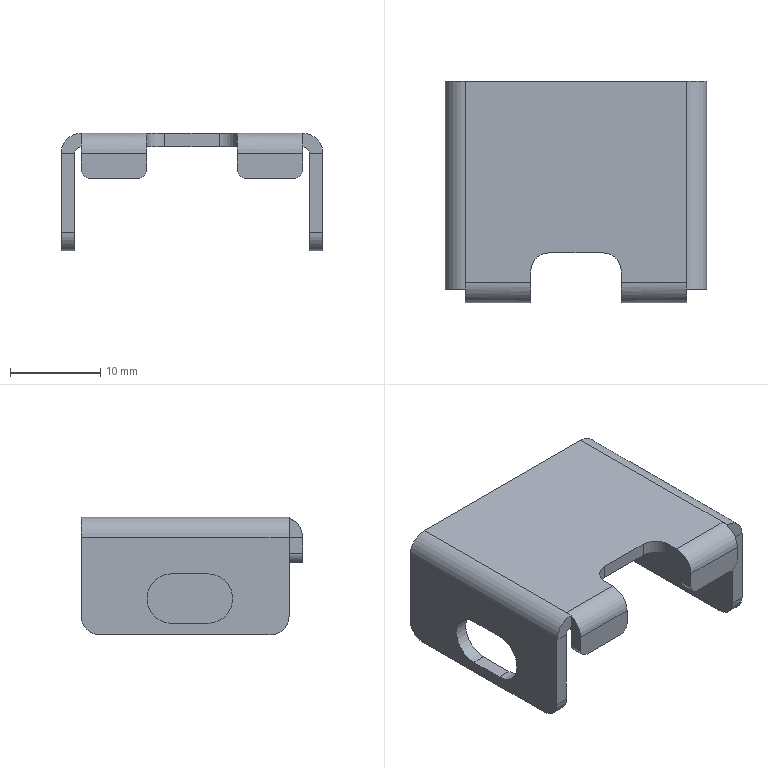Part | STEP file | 03-36 iron plate baffle (Default) | 1 solid | 54 faces | box 29 x 24.5 x 13 mm | volume 1713 mm3 | plane 34 | cylinder 20 | commonest cylinder face diameters 4 x6 1.473 x4 2 x4 4.473 x4 5.5 x2
STEP:
#1=CARTESIAN_POINT('',(5.,-13.,-2.237));
#2=VERTEX_POINT('',#1);
#3=CARTESIAN_POINT('',(5.,-10.763,0.));
#4=VERTEX_POINT('',#3);
#5=CARTESIAN_POINT('',(5.,-10.763,-2.237));
#6=DIRECTION('',(-1.,0.,0.));
#7=DIRECTION('',(0.,1.,0.));
#8=AXIS2_PLACEMENT_3D('',#5,#6,#7);
#9=CIRCLE('',#8,2.237);
#10=EDGE_CURVE('',#2,#4,#9,.T.);
#11=ORIENTED_EDGE('',*,*,#10,.F.);
#12=CARTESIAN_POINT('',(12.263,-13.,-2.237));
#13=VERTEX_POINT('',#12);
#14=CARTESIAN_POINT('',(-12.263,-13.,-2.237));
#15=DIRECTION('',(-1.,0.,0.));
#16=VECTOR('',#15,1000.);
#17=LINE('',#14,#16);
#18=EDGE_CURVE('',#13,#2,#17,.T.);
#19=ORIENTED_EDGE('',*,*,#18,.F.);
#20=CARTESIAN_POINT('',(12.263,-11.5,-0.1248));
#21=VERTEX_POINT('',#20);
#22=CARTESIAN_POINT('',(12.263,-10.763,-2.237));
#23=DIRECTION('',(1.,0.,0.));
#24=DIRECTION('',(0.,0.,1.));
#25=AXIS2_PLACEMENT_3D('',#22,#23,#24);
#26=CIRCLE('',#25,2.237);
#27=EDGE_CURVE('',#21,#13,#26,.T.);
#28=ORIENTED_EDGE('',*,*,#27,.F.);
#29=CARTESIAN_POINT('',(12.263,-10.763,0.));
#30=VERTEX_POINT('',#29);
#31=CARTESIAN_POINT('',(12.263,-10.763,-2.237));
#32=DIRECTION('',(1.,0.,0.));
#33=DIRECTION('',(0.,0.,1.));
#34=AXIS2_PLACEMENT_3D('',#31,#32,#33);
#35=CIRCLE('',#34,2.237);
#36=EDGE_CURVE('',#30,#21,#35,.T.);
#37=ORIENTED_EDGE('',*,*,#36,.F.);
#38=CARTESIAN_POINT('',(-12.263,-10.763,0.));
#39=DIRECTION('',(1.,0.,0.));
#40=VECTOR('',#39,1000.);
#41=LINE('',#38,#40);
#42=EDGE_CURVE('',#4,#30,#41,.T.);
#43=ORIENTED_EDGE('',*,*,#42,.F.);
#44=EDGE_LOOP('',(#11,#19,#28,#37,#43));
#45=FACE_OUTER_BOUND('',#44,.T.);
#46=CARTESIAN_POINT('',(-12.263,-10.763,-2.237));
#47=DIRECTION('',(-1.,0.,0.));
#48=DIRECTION('',(0.,-1.,0.));
#49=AXIS2_PLACEMENT_3D('',#46,#47,#48);
#50=CYLINDRICAL_SURFACE('',#49,2.237);
#51=ADVANCED_FACE('',(#45),#50,.T.);
#52=CARTESIAN_POINT('',(12.263,-11.5,-2.237));
#53=VERTEX_POINT('',#52);
#54=CARTESIAN_POINT('',(5.,-11.5,-2.237));
#55=VERTEX_POINT('',#54);
#56=CARTESIAN_POINT('',(12.263,-11.5,-2.237));
#57=DIRECTION('',(-1.,0.,0.));
#58=VECTOR('',#57,1000.);
#59=LINE('',#56,#58);
#60=EDGE_CURVE('',#53,#55,#59,.T.);
#61=ORIENTED_EDGE('',*,*,#60,.T.);
#62=CARTESIAN_POINT('',(5.,-10.763,-1.5));
#63=VERTEX_POINT('',#62);
#64=CARTESIAN_POINT('',(5.,-10.763,-2.237));
#65=DIRECTION('',(-1.,0.,0.));
#66=DIRECTION('',(0.,1.,0.));
#67=AXIS2_PLACEMENT_3D('',#64,#65,#66);
#68=CIRCLE('',#67,0.7366);
#69=EDGE_CURVE('',#55,#63,#68,.T.);
#70=ORIENTED_EDGE('',*,*,#69,.T.);
#71=CARTESIAN_POINT('',(12.263,-10.763,-1.5));
#72=VERTEX_POINT('',#71);
#73=CARTESIAN_POINT('',(-12.263,-10.763,-1.5));
#74=DIRECTION('',(1.,0.,0.));
#75=VECTOR('',#74,1000.);
#76=LINE('',#73,#75);
#77=EDGE_CURVE('',#63,#72,#76,.T.);
#78=ORIENTED_EDGE('',*,*,#77,.T.);
#79=CARTESIAN_POINT('',(12.263,-10.763,-2.237));
#80=DIRECTION('',(1.,0.,0.));
#81=DIRECTION('',(0.,0.,1.));
#82=AXIS2_PLACEMENT_3D('',#79,#80,#81);
#83=CIRCLE('',#82,0.7366);
#84=EDGE_CURVE('',#72,#53,#83,.T.);
#85=ORIENTED_EDGE('',*,*,#84,.T.);
#86=EDGE_LOOP('',(#61,#70,#78,#85));
#87=FACE_OUTER_BOUND('',#86,.T.);
#88=CARTESIAN_POINT('',(-12.263,-10.763,-2.237));
#89=DIRECTION('',(-1.,0.,0.));
#90=DIRECTION('',(0.,-1.,0.));
#91=AXIS2_PLACEMENT_3D('',#88,#89,#90);
#92=CYLINDRICAL_SURFACE('',#91,0.7366);
#93=ADVANCED_FACE('',(#87),#92,.F.);
#94=CARTESIAN_POINT('',(11.263,-13.,-5.));
#95=VERTEX_POINT('',#94);
#96=CARTESIAN_POINT('',(6.,-13.,-5.));
#97=VERTEX_POINT('',#96);
#98=CARTESIAN_POINT('',(-12.263,-13.,-5.));
#99=DIRECTION('',(-1.,0.,0.));
#100=VECTOR('',#99,1000.);
#101=LINE('',#98,#100);
#102=EDGE_CURVE('',#95,#97,#101,.T.);
#103=ORIENTED_EDGE('',*,*,#102,.F.);
#104=CARTESIAN_POINT('',(12.263,-13.,-4.));
#105=VERTEX_POINT('',#104);
#106=CARTESIAN_POINT('',(11.263,-13.,-4.));
#107=DIRECTION('',(0.,-1.,0.));
#108=DIRECTION('',(0.,0.,-1.));
#109=AXIS2_PLACEMENT_3D('',#106,#107,#108);
#110=CIRCLE('',#109,1.);
#111=EDGE_CURVE('',#95,#105,#110,.T.);
#112=ORIENTED_EDGE('',*,*,#111,.T.);
#113=CARTESIAN_POINT('',(12.263,-13.,-5.));
#114=DIRECTION('',(0.,0.,-1.));
#115=VECTOR('',#114,1000.);
#116=LINE('',#113,#115);
#117=EDGE_CURVE('',#13,#105,#116,.T.);
#118=ORIENTED_EDGE('',*,*,#117,.F.);
#119=ORIENTED_EDGE('',*,*,#18,.T.);
#120=CARTESIAN_POINT('',(5.,-13.,-4.));
#121=VERTEX_POINT('',#120);
#122=CARTESIAN_POINT('',(5.,-13.,-1.5));
#123=DIRECTION('',(0.,0.,1.));
#124=VECTOR('',#123,1000.);
#125=LINE('',#122,#124);
#126=EDGE_CURVE('',#121,#2,#125,.T.);
#127=ORIENTED_EDGE('',*,*,#126,.F.);
#128=CARTESIAN_POINT('',(6.,-13.,-4.));
#129=DIRECTION('',(0.,-1.,0.));
#130=DIRECTION('',(0.,0.,-1.));
#131=AXIS2_PLACEMENT_3D('',#128,#129,#130);
#132=CIRCLE('',#131,1.);
#133=EDGE_CURVE('',#121,#97,#132,.T.);
#134=ORIENTED_EDGE('',*,*,#133,.T.);
#135=EDGE_LOOP('',(#103,#112,#118,#119,#127,#134));
#136=FACE_OUTER_BOUND('',#135,.T.);
#137=CARTESIAN_POINT('',(-12.263,-13.,-1.5));
#138=DIRECTION('',(0.,-1.,0.));
#139=DIRECTION('',(0.,0.,-1.));
#140=AXIS2_PLACEMENT_3D('',#137,#138,#139);
#141=PLANE('',#140);
#142=ADVANCED_FACE('',(#136),#141,.T.);
#143=CARTESIAN_POINT('',(12.263,-11.5,-4.));
#144=VERTEX_POINT('',#143);
#145=CARTESIAN_POINT('',(12.263,-11.5,-5.));
#146=DIRECTION('',(0.,0.,-1.));
#147=VECTOR('',#146,1000.);
#148=LINE('',#145,#147);
#149=EDGE_CURVE('',#53,#144,#148,.T.);
#150=ORIENTED_EDGE('',*,*,#149,.T.);
#151=CARTESIAN_POINT('',(11.263,-11.5,-5.));
#152=VERTEX_POINT('',#151);
#153=CARTESIAN_POINT('',(11.263,-11.5,-4.));
#154=DIRECTION('',(0.,1.,0.));
#155=DIRECTION('',(0.,0.,-1.));
#156=AXIS2_PLACEMENT_3D('',#153,#154,#155);
#157=CIRCLE('',#156,1.);
#158=EDGE_CURVE('',#144,#152,#157,.T.);
#159=ORIENTED_EDGE('',*,*,#158,.T.);
#160=CARTESIAN_POINT('',(6.,-11.5,-5.));
#161=VERTEX_POINT('',#160);
#162=CARTESIAN_POINT('',(-12.263,-11.5,-5.));
#163=DIRECTION('',(-1.,0.,0.));
#164=VECTOR('',#163,1000.);
#165=LINE('',#162,#164);
#166=EDGE_CURVE('',#152,#161,#165,.T.);
#167=ORIENTED_EDGE('',*,*,#166,.T.);
#168=CARTESIAN_POINT('',(5.,-11.5,-4.));
#169=VERTEX_POINT('',#168);
#170=CARTESIAN_POINT('',(6.,-11.5,-4.));
#171=DIRECTION('',(0.,1.,0.));
#172=DIRECTION('',(0.,0.,-1.));
#173=AXIS2_PLACEMENT_3D('',#170,#171,#172);
#174=CIRCLE('',#173,1.);
#175=EDGE_CURVE('',#161,#169,#174,.T.);
#176=ORIENTED_EDGE('',*,*,#175,.T.);
#177=CARTESIAN_POINT('',(5.,-11.5,-1.5));
#178=DIRECTION('',(0.,0.,1.));
#179=VECTOR('',#178,1000.);
#180=LINE('',#177,#179);
#181=EDGE_CURVE('',#169,#55,#180,.T.);
#182=ORIENTED_EDGE('',*,*,#181,.T.);
#183=ORIENTED_EDGE('',*,*,#60,.F.);
#184=EDGE_LOOP('',(#150,#159,#167,#176,#182,#183));
#185=FACE_OUTER_BOUND('',#184,.T.);
#186=CARTESIAN_POINT('',(-12.263,-11.5,-1.5));
#187=DIRECTION('',(0.,-1.,0.));
#188=DIRECTION('',(0.,0.,-1.));
#189=AXIS2_PLACEMENT_3D('',#186,#187,#188);
#190=PLANE('',#189);
#191=ADVANCED_FACE('',(#185),#190,.F.);
#192=ORIENTED_EDGE('',*,*,#166,.F.);
#193=CARTESIAN_POINT('',(11.263,-13.,-5.));
#194=DIRECTION('',(0.,-1.,0.));
#195=VECTOR('',#194,1000.);
#196=LINE('',#193,#195);
#197=EDGE_CURVE('',#152,#95,#196,.T.);
#198=ORIENTED_EDGE('',*,*,#197,.T.);
#199=ORIENTED_EDGE('',*,*,#102,.T.);
#200=CARTESIAN_POINT('',(6.,-11.5,-5.));
#201=DIRECTION('',(0.,1.,0.));
#202=VECTOR('',#201,1000.);
#203=LINE('',#200,#202);
#204=EDGE_CURVE('',#97,#161,#203,.T.);
#205=ORIENTED_EDGE('',*,*,#204,.T.);
#206=EDGE_LOOP('',(#192,#198,#199,#205));
#207=FACE_OUTER_BOUND('',#206,.T.);
#208=CARTESIAN_POINT('',(-12.263,-13.,-5.));
#209=DIRECTION('',(0.,0.,-1.));
#210=DIRECTION('',(0.,1.,0.));
#211=AXIS2_PLACEMENT_3D('',#208,#209,#210);
#212=PLANE('',#211);
#213=ADVANCED_FACE('',(#207),#212,.T.);
#214=CARTESIAN_POINT('',(-12.263,-11.5,-0.1248));
#215=VERTEX_POINT('',#214);
#216=CARTESIAN_POINT('',(-12.263,-11.5,0.));
#217=VERTEX_POINT('',#216);
#218=CARTESIAN_POINT('',(-12.263,-11.5,-1.5));
#219=DIRECTION('',(0.,0.,1.));
#220=VECTOR('',#219,1000.);
#221=LINE('',#218,#220);
#222=EDGE_CURVE('',#215,#217,#221,.T.);
#223=ORIENTED_EDGE('',*,*,#222,.F.);
#224=CARTESIAN_POINT('',(-12.263,-10.763,0.));
#225=VERTEX_POINT('',#224);
#226=CARTESIAN_POINT('',(-12.263,-10.763,-2.237));
#227=DIRECTION('',(-1.,0.,0.));
#228=DIRECTION('',(0.,0.,1.));
#229=AXIS2_PLACEMENT_3D('',#226,#227,#228);
#230=CIRCLE('',#229,2.237);
#231=EDGE_CURVE('',#215,#225,#230,.T.);
#232=ORIENTED_EDGE('',*,*,#231,.T.);
#233=CARTESIAN_POINT('',(-12.263,11.5,0.));
#234=DIRECTION('',(0.,1.,0.));
#235=VECTOR('',#234,1000.);
#236=LINE('',#233,#235);
#237=EDGE_CURVE('',#217,#225,#236,.T.);
#238=ORIENTED_EDGE('',*,*,#237,.F.);
#239=EDGE_LOOP('',(#223,#232,#238));
#240=FACE_OUTER_BOUND('',#239,.T.);
#241=CARTESIAN_POINT('',(-12.263,-11.5,-1.5));
#242=DIRECTION('',(1.,0.,0.));
#243=DIRECTION('',(0.,1.,0.));
#244=AXIS2_PLACEMENT_3D('',#241,#242,#243);
#245=PLANE('',#244);
#246=ADVANCED_FACE('',(#240),#245,.T.);
#247=CARTESIAN_POINT('',(12.263,-11.5,0.));
#248=VERTEX_POINT('',#247);
#249=CARTESIAN_POINT('',(12.263,-11.5,0.));
#250=DIRECTION('',(0.,1.,0.));
#251=VECTOR('',#250,1000.);
#252=LINE('',#249,#251);
#253=EDGE_CURVE('',#248,#30,#252,.T.);
#254=ORIENTED_EDGE('',*,*,#253,.T.);
#255=ORIENTED_EDGE('',*,*,#36,.T.);
#256=CARTESIAN_POINT('',(12.263,-11.5,-1.5));
#257=DIRECTION('',(0.,0.,1.));
#258=VECTOR('',#257,1000.);
#259=LINE('',#256,#258);
#260=EDGE_CURVE('',#21,#248,#259,.T.);
#261=ORIENTED_EDGE('',*,*,#260,.T.);
#262=EDGE_LOOP('',(#254,#255,#261));
#263=FACE_OUTER_BOUND('',#262,.T.);
#264=CARTESIAN_POINT('',(12.263,-10.763,-1.5));
#265=DIRECTION('',(-1.,0.,0.));
#266=DIRECTION('',(0.,-1.,0.));
#267=AXIS2_PLACEMENT_3D('',#264,#265,#266);
#268=PLANE('',#267);
#269=ADVANCED_FACE('',(#263),#268,.T.);
#270=ORIENTED_EDGE('',*,*,#77,.F.);
#271=CARTESIAN_POINT('',(5.,-9.5,-1.5));
#272=VERTEX_POINT('',#271);
#273=CARTESIAN_POINT('',(5.,-11.5,-1.5));
#274=DIRECTION('',(0.,1.,0.));
#275=VECTOR('',#274,1000.);
#276=LINE('',#273,#275);
#277=EDGE_CURVE('',#63,#272,#276,.T.);
#278=ORIENTED_EDGE('',*,*,#277,.T.);
#279=CARTESIAN_POINT('',(3.,-7.5,-1.5));
#280=VERTEX_POINT('',#279);
#281=CARTESIAN_POINT('',(3.,-9.5,-1.5));
#282=DIRECTION('',(0.,0.,1.));
#283=DIRECTION('',(1.,0.,0.));
#284=AXIS2_PLACEMENT_3D('',#281,#282,#283);
#285=CIRCLE('',#284,2.);
#286=EDGE_CURVE('',#272,#280,#285,.T.);
#287=ORIENTED_EDGE('',*,*,#286,.T.);
#288=CARTESIAN_POINT('',(-3.,-7.5,-1.5));
#289=VERTEX_POINT('',#288);
#290=CARTESIAN_POINT('',(13.,-7.5,-1.5));
#291=DIRECTION('',(-1.,0.,0.));
#292=VECTOR('',#291,1000.);
#293=LINE('',#290,#292);
#294=EDGE_CURVE('',#280,#289,#293,.T.);
#295=ORIENTED_EDGE('',*,*,#294,.T.);
#296=CARTESIAN_POINT('',(-5.,-9.5,-1.5));
#297=VERTEX_POINT('',#296);
#298=CARTESIAN_POINT('',(-3.,-9.5,-1.5));
#299=DIRECTION('',(0.,0.,1.));
#300=DIRECTION('',(1.,0.,0.));
#301=AXIS2_PLACEMENT_3D('',#298,#299,#300);
#302=CIRCLE('',#301,2.);
#303=EDGE_CURVE('',#289,#297,#302,.T.);
#304=ORIENTED_EDGE('',*,*,#303,.T.);
#305=CARTESIAN_POINT('',(-5.,-10.763,-1.5));
#306=VERTEX_POINT('',#305);
#307=CARTESIAN_POINT('',(-5.,-11.5,-1.5));
#308=DIRECTION('',(0.,-1.,0.));
#309=VECTOR('',#308,1000.);
#310=LINE('',#307,#309);
#311=EDGE_CURVE('',#297,#306,#310,.T.);
#312=ORIENTED_EDGE('',*,*,#311,.T.);
#313=CARTESIAN_POINT('',(-12.263,-10.763,-1.5));
#314=VERTEX_POINT('',#313);
#315=CARTESIAN_POINT('',(-12.263,-10.763,-1.5));
#316=DIRECTION('',(1.,0.,0.));
#317=VECTOR('',#316,1000.);
#318=LINE('',#315,#317);
#319=EDGE_CURVE('',#314,#306,#318,.T.);
#320=ORIENTED_EDGE('',*,*,#319,.F.);
#321=CARTESIAN_POINT('',(-12.263,11.5,-1.5));
#322=VERTEX_POINT('',#321);
#323=CARTESIAN_POINT('',(-12.263,11.5,-1.5));
#324=DIRECTION('',(0.,-1.,0.));
#325=VECTOR('',#324,1000.);
#326=LINE('',#323,#325);
#327=EDGE_CURVE('',#322,#314,#326,.T.);
#328=ORIENTED_EDGE('',*,*,#327,.F.);
#329=CARTESIAN_POINT('',(12.263,11.5,-1.5));
#330=VERTEX_POINT('',#329);
#331=CARTESIAN_POINT('',(-13.,11.5,-1.5));
#332=DIRECTION('',(-1.,0.,0.));
#333=VECTOR('',#332,1000.);
#334=LINE('',#331,#333);
#335=EDGE_CURVE('',#330,#322,#334,.T.);
#336=ORIENTED_EDGE('',*,*,#335,.F.);
#337=CARTESIAN_POINT('',(12.263,-11.5,-1.5));
#338=DIRECTION('',(0.,1.,0.));
#339=VECTOR('',#338,1000.);
#340=LINE('',#337,#339);
#341=EDGE_CURVE('',#72,#330,#340,.T.);
#342=ORIENTED_EDGE('',*,*,#341,.F.);
#343=EDGE_LOOP('',(#270,#278,#287,#295,#304,#312,#320,#328,#336,#342));
#344=FACE_OUTER_BOUND('',#343,.T.);
#345=CARTESIAN_POINT('',(13.,-11.5,-1.5));
#346=DIRECTION('',(0.,0.,1.));
#347=DIRECTION('',(1.,0.,0.));
#348=AXIS2_PLACEMENT_3D('',#345,#346,#347);
#349=PLANE('',#348);
#350=ADVANCED_FACE('',(#344),#349,.F.);
#351=CARTESIAN_POINT('',(5.,-9.5,0.));
#352=VERTEX_POINT('',#351);
#353=CARTESIAN_POINT('',(5.,-9.5,0.));
#354=DIRECTION('',(0.,1.,0.));
#355=VECTOR('',#354,1000.);
#356=LINE('',#353,#355);
#357=EDGE_CURVE('',#4,#352,#356,.T.);
#358=ORIENTED_EDGE('',*,*,#357,.F.);
#359=ORIENTED_EDGE('',*,*,#42,.T.);
#360=CARTESIAN_POINT('',(12.263,11.5,0.));
#361=VERTEX_POINT('',#360);
#362=CARTESIAN_POINT('',(12.263,-11.5,0.));
#363=DIRECTION('',(0.,1.,0.));
#364=VECTOR('',#363,1000.);
#365=LINE('',#362,#364);
#366=EDGE_CURVE('',#30,#361,#365,.T.);
#367=ORIENTED_EDGE('',*,*,#366,.T.);
#368=CARTESIAN_POINT('',(-12.263,11.5,0.));
#369=VERTEX_POINT('',#368);
#370=CARTESIAN_POINT('',(-13.,11.5,0.));
#371=DIRECTION('',(-1.,0.,0.));
#372=VECTOR('',#371,1000.);
#373=LINE('',#370,#372);
#374=EDGE_CURVE('',#361,#369,#373,.T.);
#375=ORIENTED_EDGE('',*,*,#374,.T.);
#376=CARTESIAN_POINT('',(-12.263,11.5,0.));
#377=DIRECTION('',(0.,-1.,0.));
#378=VECTOR('',#377,1000.);
#379=LINE('',#376,#378);
#380=EDGE_CURVE('',#369,#225,#379,.T.);
#381=ORIENTED_EDGE('',*,*,#380,.T.);
#382=CARTESIAN_POINT('',(-5.,-10.763,0.));
#383=VERTEX_POINT('',#382);
#384=CARTESIAN_POINT('',(-12.263,-10.763,0.));
#385=DIRECTION('',(1.,0.,0.));
#386=VECTOR('',#385,1000.);
#387=LINE('',#384,#386);
#388=EDGE_CURVE('',#225,#383,#387,.T.);
#389=ORIENTED_EDGE('',*,*,#388,.T.);
#390=CARTESIAN_POINT('',(-5.,-9.5,0.));
#391=VERTEX_POINT('',#390);
#392=CARTESIAN_POINT('',(-5.,-9.5,0.));
#393=DIRECTION('',(0.,-1.,0.));
#394=VECTOR('',#393,1000.);
#395=LINE('',#392,#394);
#396=EDGE_CURVE('',#391,#383,#395,.T.);
#397=ORIENTED_EDGE('',*,*,#396,.F.);
#398=CARTESIAN_POINT('',(-3.,-7.5,0.));
#399=VERTEX_POINT('',#398);
#400=CARTESIAN_POINT('',(-3.,-9.5,0.));
#401=DIRECTION('',(0.,0.,1.));
#402=DIRECTION('',(-1.,0.,0.));
#403=AXIS2_PLACEMENT_3D('',#400,#401,#402);
#404=CIRCLE('',#403,2.);
#405=EDGE_CURVE('',#399,#391,#404,.T.);
#406=ORIENTED_EDGE('',*,*,#405,.F.);
#407=CARTESIAN_POINT('',(3.,-7.5,0.));
#408=VERTEX_POINT('',#407);
#409=CARTESIAN_POINT('',(-3.,-7.5,0.));
#410=DIRECTION('',(-1.,0.,0.));
#411=VECTOR('',#410,1000.);
#412=LINE('',#409,#411);
#413=EDGE_CURVE('',#408,#399,#412,.T.);
#414=ORIENTED_EDGE('',*,*,#413,.F.);
#415=CARTESIAN_POINT('',(3.,-9.5,0.));
#416=DIRECTION('',(0.,0.,1.));
#417=DIRECTION('',(1.,0.,0.));
#418=AXIS2_PLACEMENT_3D('',#415,#416,#417);
#419=CIRCLE('',#418,2.);
#420=EDGE_CURVE('',#352,#408,#419,.T.);
#421=ORIENTED_EDGE('',*,*,#420,.F.);
#422=EDGE_LOOP('',(#358,#359,#367,#375,#381,#389,#397,#406,#414,#421));
#423=FACE_OUTER_BOUND('',#422,.T.);
#424=CARTESIAN_POINT('',(13.,-11.5,0.));
#425=DIRECTION('',(0.,0.,1.));
#426=DIRECTION('',(1.,0.,0.));
#427=AXIS2_PLACEMENT_3D('',#424,#425,#426);
#428=PLANE('',#427);
#429=ADVANCED_FACE('',(#423),#428,.T.);
#430=ORIENTED_EDGE('',*,*,#335,.T.);
#431=CARTESIAN_POINT('',(-12.263,11.5,-1.5));
#432=DIRECTION('',(0.,0.,1.));
#433=VECTOR('',#432,1000.);
#434=LINE('',#431,#433);
#435=EDGE_CURVE('',#322,#369,#434,.T.);
#436=ORIENTED_EDGE('',*,*,#435,.T.);
#437=ORIENTED_EDGE('',*,*,#374,.F.);
#438=CARTESIAN_POINT('',(12.263,11.5,-1.5));
#439=DIRECTION('',(0.,0.,1.));
#440=VECTOR('',#439,1000.);
#441=LINE('',#438,#440);
#442=EDGE_CURVE('',#330,#361,#441,.T.);
#443=ORIENTED_EDGE('',*,*,#442,.F.);
#444=EDGE_LOOP('',(#430,#436,#437,#443));
#445=FACE_OUTER_BOUND('',#444,.T.);
#446=CARTESIAN_POINT('',(-13.,11.5,-1.5));
#447=DIRECTION('',(0.,1.,0.));
#448=DIRECTION('',(0.,0.,1.));
#449=AXIS2_PLACEMENT_3D('',#446,#447,#448);
#450=PLANE('',#449);
#451=ADVANCED_FACE('',(#445),#450,.T.);
#452=CARTESIAN_POINT('',(13.,11.5,-2.237));
#453=VERTEX_POINT('',#452);
#454=CARTESIAN_POINT('',(14.5,11.5,-2.237));
#455=VERTEX_POINT('',#454);
#456=CARTESIAN_POINT('',(13.,11.5,-2.237));
#457=DIRECTION('',(1.,0.,0.));
#458=VECTOR('',#457,1000.);
#459=LINE('',#456,#458);
#460=EDGE_CURVE('',#453,#455,#459,.T.);
#461=ORIENTED_EDGE('',*,*,#460,.F.);
#462=CARTESIAN_POINT('',(12.263,11.5,-2.237));
#463=DIRECTION('',(0.,1.,0.));
#464=DIRECTION('',(0.,0.,-1.));
#465=AXIS2_PLACEMENT_3D('',#462,#463,#464);
#466=CIRCLE('',#465,0.7366);
#467=EDGE_CURVE('',#330,#453,#466,.T.);
#468=ORIENTED_EDGE('',*,*,#467,.F.);
#469=ORIENTED_EDGE('',*,*,#442,.T.);
#470=CARTESIAN_POINT('',(12.263,11.5,-2.237));
#471=DIRECTION('',(0.,1.,0.));
#472=DIRECTION('',(0.,0.,-1.));
#473=AXIS2_PLACEMENT_3D('',#470,#471,#472);
#474=CIRCLE('',#473,2.237);
#475=EDGE_CURVE('',#361,#455,#474,.T.);
#476=ORIENTED_EDGE('',*,*,#475,.T.);
#477=EDGE_LOOP('',(#461,#468,#469,#476));
#478=FACE_OUTER_BOUND('',#477,.T.);
#479=CARTESIAN_POINT('',(12.263,11.5,-2.237));
#480=DIRECTION('',(0.,1.,0.));
#481=DIRECTION('',(0.,0.,1.));
#482=AXIS2_PLACEMENT_3D('',#479,#480,#481);
#483=PLANE('',#482);
#484=ADVANCED_FACE('',(#478),#483,.T.);
#485=CARTESIAN_POINT('',(13.,-11.5,-2.237));
#486=VERTEX_POINT('',#485);
#487=CARTESIAN_POINT('',(12.263,-11.5,-1.5));
#488=VERTEX_POINT('',#487);
#489=CARTESIAN_POINT('',(12.263,-11.5,-2.237));
#490=DIRECTION('',(0.,-1.,0.));
#491=DIRECTION('',(0.,0.,-1.));
#492=AXIS2_PLACEMENT_3D('',#489,#490,#491);
#493=CIRCLE('',#492,0.7366);
#494=EDGE_CURVE('',#486,#488,#493,.T.);
#495=ORIENTED_EDGE('',*,*,#494,.F.);
#496=CARTESIAN_POINT('',(14.5,-11.5,-2.237));
#497=VERTEX_POINT('',#496);
#498=CARTESIAN_POINT('',(13.,-11.5,-2.237));
#499=DIRECTION('',(1.,0.,0.));
#500=VECTOR('',#499,1000.);
#501=LINE('',#498,#500);
#502=EDGE_CURVE('',#486,#497,#501,.T.);
#503=ORIENTED_EDGE('',*,*,#502,.T.);
#504=CARTESIAN_POINT('',(12.263,-11.5,-2.237));
#505=DIRECTION('',(0.,-1.,0.));
#506=DIRECTION('',(0.,0.,-1.));
#507=AXIS2_PLACEMENT_3D('',#504,#505,#506);
#508=CIRCLE('',#507,2.237);
#509=EDGE_CURVE('',#497,#248,#508,.T.);
#510=ORIENTED_EDGE('',*,*,#509,.T.);
#511=ORIENTED_EDGE('',*,*,#260,.F.);
#512=CARTESIAN_POINT('',(12.263,-11.5,-1.5));
#513=DIRECTION('',(0.,0.,1.));
#514=VECTOR('',#513,1000.);
#515=LINE('',#512,#514);
#516=EDGE_CURVE('',#488,#21,#515,.T.);
#517=ORIENTED_EDGE('',*,*,#516,.F.);
#518=EDGE_LOOP('',(#495,#503,#510,#511,#517));
#519=FACE_OUTER_BOUND('',#518,.T.);
#520=CARTESIAN_POINT('',(12.263,-11.5,-2.237));
#521=DIRECTION('',(0.,1.,0.));
#522=DIRECTION('',(0.,0.,1.));
#523=AXIS2_PLACEMENT_3D('',#520,#521,#522);
#524=PLANE('',#523);
#525=ADVANCED_FACE('',(#519),#524,.F.);
#526=ORIENTED_EDGE('',*,*,#253,.F.);
#527=ORIENTED_EDGE('',*,*,#509,.F.);
#528=CARTESIAN_POINT('',(14.5,-11.5,-2.237));
#529=DIRECTION('',(0.,-1.,0.));
#530=VECTOR('',#529,1000.);
#531=LINE('',#528,#530);
#532=EDGE_CURVE('',#455,#497,#531,.T.);
#533=ORIENTED_EDGE('',*,*,#532,.F.);
#534=ORIENTED_EDGE('',*,*,#475,.F.);
#535=ORIENTED_EDGE('',*,*,#366,.F.);
#536=EDGE_LOOP('',(#526,#527,#533,#534,#535));
#537=FACE_OUTER_BOUND('',#536,.T.);
#538=CARTESIAN_POINT('',(12.263,-11.5,-2.237));
#539=DIRECTION('',(0.,-1.,0.));
#540=DIRECTION('',(1.,0.,0.));
#541=AXIS2_PLACEMENT_3D('',#538,#539,#540);
#542=CYLINDRICAL_SURFACE('',#541,2.237);
#543=ADVANCED_FACE('',(#537),#542,.T.);
#544=CARTESIAN_POINT('',(12.263,-11.5,-1.5));
#545=DIRECTION('',(0.,1.,0.));
#546=VECTOR('',#545,1000.);
#547=LINE('',#544,#546);
#548=EDGE_CURVE('',#488,#72,#547,.T.);
#549=ORIENTED_EDGE('',*,*,#548,.T.);
#550=ORIENTED_EDGE('',*,*,#341,.T.);
#551=ORIENTED_EDGE('',*,*,#467,.T.);
#552=CARTESIAN_POINT('',(13.,11.5,-2.237));
#553=DIRECTION('',(0.,-1.,0.));
#554=VECTOR('',#553,1000.);
#555=LINE('',#552,#554);
#556=EDGE_CURVE('',#453,#486,#555,.T.);
#557=ORIENTED_EDGE('',*,*,#556,.T.);
#558=ORIENTED_EDGE('',*,*,#494,.T.);
#559=EDGE_LOOP('',(#549,#550,#551,#557,#558));
#560=FACE_OUTER_BOUND('',#559,.T.);
#561=CARTESIAN_POINT('',(12.263,-11.5,-2.237));
#562=DIRECTION('',(0.,-1.,0.));
#563=DIRECTION('',(1.,0.,0.));
#564=AXIS2_PLACEMENT_3D('',#561,#562,#563);
#565=CYLINDRICAL_SURFACE('',#564,0.7366);
#566=ADVANCED_FACE('',(#560),#565,.F.);
#567=CARTESIAN_POINT('',(13.,-11.5,-11.));
#568=VERTEX_POINT('',#567);
#569=CARTESIAN_POINT('',(13.,-11.5,-1.5));
#570=DIRECTION('',(0.,0.,1.));
#571=VECTOR('',#570,1000.);
#572=LINE('',#569,#571);
#573=EDGE_CURVE('',#568,#486,#572,.T.);
#574=ORIENTED_EDGE('',*,*,#573,.F.);
#575=CARTESIAN_POINT('',(14.5,-11.5,-11.));
#576=VERTEX_POINT('',#575);
#577=CARTESIAN_POINT('',(14.5,-11.5,-11.));
#578=DIRECTION('',(1.,0.,0.));
#579=VECTOR('',#578,1000.);
#580=LINE('',#577,#579);
#581=EDGE_CURVE('',#568,#576,#580,.T.);
#582=ORIENTED_EDGE('',*,*,#581,.T.);
#583=CARTESIAN_POINT('',(14.5,-11.5,-1.5));
#584=DIRECTION('',(0.,0.,1.));
#585=VECTOR('',#584,1000.);
#586=LINE('',#583,#585);
#587=EDGE_CURVE('',#576,#497,#586,.T.);
#588=ORIENTED_EDGE('',*,*,#587,.T.);
#589=ORIENTED_EDGE('',*,*,#502,.F.);
#590=EDGE_LOOP('',(#574,#582,#588,#589));
#591=FACE_OUTER_BOUND('',#590,.T.);
#592=CARTESIAN_POINT('',(14.5,-11.5,-1.5));
#593=DIRECTION('',(0.,-1.,0.));
#594=DIRECTION('',(1.,0.,0.));
#595=AXIS2_PLACEMENT_3D('',#592,#593,#594);
#596=PLANE('',#595);
#597=ADVANCED_FACE('',(#591),#596,.T.);
#598=CARTESIAN_POINT('',(14.5,11.5,-11.));
#599=VERTEX_POINT('',#598);
#600=CARTESIAN_POINT('',(14.5,11.5,-13.));
#601=DIRECTION('',(0.,0.,-1.));
#602=VECTOR('',#601,1000.);
#603=LINE('',#600,#602);
#604=EDGE_CURVE('',#455,#599,#603,.T.);
#605=ORIENTED_EDGE('',*,*,#604,.T.);
#606=CARTESIAN_POINT('',(13.,11.5,-11.));
#607=VERTEX_POINT('',#606);
#608=CARTESIAN_POINT('',(14.5,11.5,-11.));
#609=DIRECTION('',(-1.,0.,0.));
#610=VECTOR('',#609,1000.);
#611=LINE('',#608,#610);
#612=EDGE_CURVE('',#599,#607,#611,.T.);
#613=ORIENTED_EDGE('',*,*,#612,.T.);
#614=CARTESIAN_POINT('',(13.,11.5,-13.));
#615=DIRECTION('',(0.,0.,-1.));
#616=VECTOR('',#615,1000.);
#617=LINE('',#614,#616);
#618=EDGE_CURVE('',#453,#607,#617,.T.);
#619=ORIENTED_EDGE('',*,*,#618,.F.);
#620=ORIENTED_EDGE('',*,*,#460,.T.);
#621=EDGE_LOOP('',(#605,#613,#619,#620));
#622=FACE_OUTER_BOUND('',#621,.T.);
#623=CARTESIAN_POINT('',(14.5,11.5,-13.));
#624=DIRECTION('',(0.,1.,0.));
#625=DIRECTION('',(0.,0.,1.));
#626=AXIS2_PLACEMENT_3D('',#623,#624,#625);
#627=PLANE('',#626);
#628=ADVANCED_FACE('',(#622),#627,.T.);
#629=ORIENTED_EDGE('',*,*,#587,.F.);
#630=CARTESIAN_POINT('',(14.5,-9.5,-13.));
#631=VERTEX_POINT('',#630);
#632=CARTESIAN_POINT('',(14.5,-9.5,-11.));
#633=DIRECTION('',(1.,0.,0.));
#634=DIRECTION('',(0.,0.,-1.));
#635=AXIS2_PLACEMENT_3D('',#632,#633,#634);
#636=CIRCLE('',#635,2.);
#637=EDGE_CURVE('',#576,#631,#636,.T.);
#638=ORIENTED_EDGE('',*,*,#637,.T.);
#639=CARTESIAN_POINT('',(14.5,9.5,-13.));
#640=VERTEX_POINT('',#639);
#641=CARTESIAN_POINT('',(14.5,-11.5,-13.));
#642=DIRECTION('',(0.,-1.,0.));
#643=VECTOR('',#642,1000.);
#644=LINE('',#641,#643);
#645=EDGE_CURVE('',#640,#631,#644,.T.);
#646=ORIENTED_EDGE('',*,*,#645,.F.);
#647=CARTESIAN_POINT('',(14.5,9.5,-11.));
#648=DIRECTION('',(1.,0.,0.));
#649=DIRECTION('',(0.,0.,-1.));
#650=AXIS2_PLACEMENT_3D('',#647,#648,#649);
#651=CIRCLE('',#650,2.);
#652=EDGE_CURVE('',#640,#599,#651,.T.);
#653=ORIENTED_EDGE('',*,*,#652,.T.);
#654=ORIENTED_EDGE('',*,*,#604,.F.);
#655=ORIENTED_EDGE('',*,*,#532,.T.);
#656=EDGE_LOOP('',(#629,#638,#646,#653,#654,#655));
#657=FACE_OUTER_BOUND('',#656,.T.);
#658=CARTESIAN_POINT('',(14.5,-11.5,-1.5));
#659=DIRECTION('',(1.,0.,0.));
#660=DIRECTION('',(0.,0.,-1.));
#661=AXIS2_PLACEMENT_3D('',#658,#659,#660);
#662=PLANE('',#661);
#663=ADVANCED_FACE('',(#657),#662,.T.);
#664=CARTESIAN_POINT('',(13.,9.5,-13.));
#665=VERTEX_POINT('',#664);
#666=CARTESIAN_POINT('',(13.,-9.5,-13.));
#667=VERTEX_POINT('',#666);
#668=CARTESIAN_POINT('',(13.,-11.5,-13.));
#669=DIRECTION('',(0.,-1.,0.));
#670=VECTOR('',#669,1000.);
#671=LINE('',#668,#670);
#672=EDGE_CURVE('',#665,#667,#671,.T.);
#673=ORIENTED_EDGE('',*,*,#672,.T.);
#674=CARTESIAN_POINT('',(13.,-9.5,-11.));
#675=DIRECTION('',(-1.,0.,0.));
#676=DIRECTION('',(0.,0.,-1.));
#677=AXIS2_PLACEMENT_3D('',#674,#675,#676);
#678=CIRCLE('',#677,2.);
#679=EDGE_CURVE('',#667,#568,#678,.T.);
#680=ORIENTED_EDGE('',*,*,#679,.T.);
#681=ORIENTED_EDGE('',*,*,#573,.T.);
#682=ORIENTED_EDGE('',*,*,#556,.F.);
#683=ORIENTED_EDGE('',*,*,#618,.T.);
#684=CARTESIAN_POINT('',(13.,9.5,-11.));
#685=DIRECTION('',(-1.,0.,0.));
#686=DIRECTION('',(0.,0.,-1.));
#687=AXIS2_PLACEMENT_3D('',#684,#685,#686);
#688=CIRCLE('',#687,2.);
#689=EDGE_CURVE('',#607,#665,#688,.T.);
#690=ORIENTED_EDGE('',*,*,#689,.T.);
#691=EDGE_LOOP('',(#673,#680,#681,#682,#683,#690));
#692=FACE_OUTER_BOUND('',#691,.T.);
#693=CARTESIAN_POINT('',(13.,-11.5,-1.5));
#694=DIRECTION('',(1.,0.,0.));
#695=DIRECTION('',(0.,0.,-1.));
#696=AXIS2_PLACEMENT_3D('',#693,#694,#695);
#697=PLANE('',#696);
#698=ADVANCED_FACE('',(#692),#697,.F.);
#699=ORIENTED_EDGE('',*,*,#645,.T.);
#700=CARTESIAN_POINT('',(14.5,-9.5,-13.));
#701=DIRECTION('',(-1.,0.,0.));
#702=VECTOR('',#701,1000.);
#703=LINE('',#700,#702);
#704=EDGE_CURVE('',#631,#667,#703,.T.);
#705=ORIENTED_EDGE('',*,*,#704,.T.);
#706=ORIENTED_EDGE('',*,*,#672,.F.);
#707=CARTESIAN_POINT('',(14.5,9.5,-13.));
#708=DIRECTION('',(1.,0.,0.));
#709=VECTOR('',#708,1000.);
#710=LINE('',#707,#709);
#711=EDGE_CURVE('',#665,#640,#710,.T.);
#712=ORIENTED_EDGE('',*,*,#711,.T.);
#713=EDGE_LOOP('',(#699,#705,#706,#712));
#714=FACE_OUTER_BOUND('',#713,.T.);
#715=CARTESIAN_POINT('',(14.5,-11.5,-13.));
#716=DIRECTION('',(0.,0.,-1.));
#717=DIRECTION('',(-1.,0.,0.));
#718=AXIS2_PLACEMENT_3D('',#715,#716,#717);
#719=PLANE('',#718);
#720=ADVANCED_FACE('',(#714),#719,.T.);
#721=CARTESIAN_POINT('',(-13.,-11.5,-2.237));
#722=VERTEX_POINT('',#721);
#723=CARTESIAN_POINT('',(-14.5,-11.5,-2.237));
#724=VERTEX_POINT('',#723);
#725=CARTESIAN_POINT('',(-13.,-11.5,-2.237));
#726=DIRECTION('',(-1.,0.,0.));
#727=VECTOR('',#726,1000.);
#728=LINE('',#725,#727);
#729=EDGE_CURVE('',#722,#724,#728,.T.);
#730=ORIENTED_EDGE('',*,*,#729,.F.);
#731=CARTESIAN_POINT('',(-12.263,-11.5,-1.5));
#732=VERTEX_POINT('',#731);
#733=CARTESIAN_POINT('',(-12.263,-11.5,-2.237));
#734=DIRECTION('',(0.,-1.,0.));
#735=DIRECTION('',(0.,0.,1.));
#736=AXIS2_PLACEMENT_3D('',#733,#734,#735);
#737=CIRCLE('',#736,0.7366);
#738=EDGE_CURVE('',#732,#722,#737,.T.);
#739=ORIENTED_EDGE('',*,*,#738,.F.);
#740=CARTESIAN_POINT('',(-12.263,-11.5,-1.5));
#741=DIRECTION('',(0.,0.,1.));
#742=VECTOR('',#741,1000.);
#743=LINE('',#740,#742);
#744=EDGE_CURVE('',#732,#215,#743,.T.);
#745=ORIENTED_EDGE('',*,*,#744,.T.);
#746=ORIENTED_EDGE('',*,*,#222,.T.);
#747=CARTESIAN_POINT('',(-12.263,-11.5,-2.237));
#748=DIRECTION('',(0.,-1.,0.));
#749=DIRECTION('',(0.,0.,1.));
#750=AXIS2_PLACEMENT_3D('',#747,#748,#749);
#751=CIRCLE('',#750,2.237);
#752=EDGE_CURVE('',#217,#724,#751,.T.);
#753=ORIENTED_EDGE('',*,*,#752,.T.);
#754=EDGE_LOOP('',(#730,#739,#745,#746,#753));
#755=FACE_OUTER_BOUND('',#754,.T.);
#756=CARTESIAN_POINT('',(-12.263,-11.5,-2.237));
#757=DIRECTION('',(0.,-1.,0.));
#758=DIRECTION('',(0.,0.,-1.));
#759=AXIS2_PLACEMENT_3D('',#756,#757,#758);
#760=PLANE('',#759);
#761=ADVANCED_FACE('',(#755),#760,.T.);
#762=CARTESIAN_POINT('',(-13.,11.5,-2.237));
#763=VERTEX_POINT('',#762);
#764=CARTESIAN_POINT('',(-12.263,11.5,-2.237));
#765=DIRECTION('',(0.,1.,0.));
#766=DIRECTION('',(0.,0.,1.));
#767=AXIS2_PLACEMENT_3D('',#764,#765,#766);
#768=CIRCLE('',#767,0.7366);
#769=EDGE_CURVE('',#763,#322,#768,.T.);
#770=ORIENTED_EDGE('',*,*,#769,.F.);
#771=CARTESIAN_POINT('',(-14.5,11.5,-2.237));
#772=VERTEX_POINT('',#771);
#773=CARTESIAN_POINT('',(-13.,11.5,-2.237));
#774=DIRECTION('',(-1.,0.,0.));
#775=VECTOR('',#774,1000.);
#776=LINE('',#773,#775);
#777=EDGE_CURVE('',#763,#772,#776,.T.);
#778=ORIENTED_EDGE('',*,*,#777,.T.);
#779=CARTESIAN_POINT('',(-12.263,11.5,-2.237));
#780=DIRECTION('',(0.,1.,0.));
#781=DIRECTION('',(0.,0.,1.));
#782=AXIS2_PLACEMENT_3D('',#779,#780,#781);
#783=CIRCLE('',#782,2.237);
#784=EDGE_CURVE('',#772,#369,#783,.T.);
#785=ORIENTED_EDGE('',*,*,#784,.T.);
#786=ORIENTED_EDGE('',*,*,#435,.F.);
#787=EDGE_LOOP('',(#770,#778,#785,#786));
#788=FACE_OUTER_BOUND('',#787,.T.);
#789=CARTESIAN_POINT('',(-12.263,11.5,-2.237));
#790=DIRECTION('',(0.,-1.,0.));
#791=DIRECTION('',(0.,0.,-1.));
#792=AXIS2_PLACEMENT_3D('',#789,#790,#791);
#793=PLANE('',#792);
#794=ADVANCED_FACE('',(#788),#793,.F.);
#795=ORIENTED_EDGE('',*,*,#380,.F.);
#796=ORIENTED_EDGE('',*,*,#784,.F.);
#797=CARTESIAN_POINT('',(-14.5,-11.5,-2.237));
#798=DIRECTION('',(0.,-1.,0.));
#799=VECTOR('',#798,1000.);
#800=LINE('',#797,#799);
#801=EDGE_CURVE('',#772,#724,#800,.T.);
#802=ORIENTED_EDGE('',*,*,#801,.T.);
#803=ORIENTED_EDGE('',*,*,#752,.F.);
#804=ORIENTED_EDGE('',*,*,#237,.T.);
#805=EDGE_LOOP('',(#795,#796,#802,#803,#804));
#806=FACE_OUTER_BOUND('',#805,.T.);
#807=CARTESIAN_POINT('',(-12.263,11.5,-2.237));
#808=DIRECTION('',(0.,1.,0.));
#809=DIRECTION('',(-1.,0.,0.));
#810=AXIS2_PLACEMENT_3D('',#807,#808,#809);
#811=CYLINDRICAL_SURFACE('',#810,2.237);
#812=ADVANCED_FACE('',(#806),#811,.T.);
#813=ORIENTED_EDGE('',*,*,#327,.T.);
#814=CARTESIAN_POINT('',(-12.263,-11.5,-1.5));
#815=DIRECTION('',(0.,1.,0.));
#816=VECTOR('',#815,1000.);
#817=LINE('',#814,#816);
#818=EDGE_CURVE('',#732,#314,#817,.T.);
#819=ORIENTED_EDGE('',*,*,#818,.F.);
#820=ORIENTED_EDGE('',*,*,#738,.T.);
#821=CARTESIAN_POINT('',(-13.,-11.5,-2.237));
#822=DIRECTION('',(0.,1.,0.));
#823=VECTOR('',#822,1000.);
#824=LINE('',#821,#823);
#825=EDGE_CURVE('',#722,#763,#824,.T.);
#826=ORIENTED_EDGE('',*,*,#825,.T.);
#827=ORIENTED_EDGE('',*,*,#769,.T.);
#828=EDGE_LOOP('',(#813,#819,#820,#826,#827));
#829=FACE_OUTER_BOUND('',#828,.T.);
#830=CARTESIAN_POINT('',(-12.263,11.5,-2.237));
#831=DIRECTION('',(0.,1.,0.));
#832=DIRECTION('',(-1.,0.,0.));
#833=AXIS2_PLACEMENT_3D('',#830,#831,#832);
#834=CYLINDRICAL_SURFACE('',#833,0.7366);
#835=ADVANCED_FACE('',(#829),#834,.F.);
#836=CARTESIAN_POINT('',(-14.5,-11.5,-11.));
#837=VERTEX_POINT('',#836);
#838=CARTESIAN_POINT('',(-14.5,-11.5,-1.5));
#839=DIRECTION('',(0.,0.,-1.));
#840=VECTOR('',#839,1000.);
#841=LINE('',#838,#840);
#842=EDGE_CURVE('',#724,#837,#841,.T.);
#843=ORIENTED_EDGE('',*,*,#842,.T.);
#844=CARTESIAN_POINT('',(-13.,-11.5,-11.));
#845=VERTEX_POINT('',#844);
#846=CARTESIAN_POINT('',(-14.5,-11.5,-11.));
#847=DIRECTION('',(1.,0.,0.));
#848=VECTOR('',#847,1000.);
#849=LINE('',#846,#848);
#850=EDGE_CURVE('',#837,#845,#849,.T.);
#851=ORIENTED_EDGE('',*,*,#850,.T.);
#852=CARTESIAN_POINT('',(-13.,-11.5,-1.5));
#853=DIRECTION('',(0.,0.,-1.));
#854=VECTOR('',#853,1000.);
#855=LINE('',#852,#854);
#856=EDGE_CURVE('',#722,#845,#855,.T.);
#857=ORIENTED_EDGE('',*,*,#856,.F.);
#858=ORIENTED_EDGE('',*,*,#729,.T.);
#859=EDGE_LOOP('',(#843,#851,#857,#858));
#860=FACE_OUTER_BOUND('',#859,.T.);
#861=CARTESIAN_POINT('',(-14.5,-11.5,-1.5));
#862=DIRECTION('',(0.,-1.,0.));
#863=DIRECTION('',(1.,0.,0.));
#864=AXIS2_PLACEMENT_3D('',#861,#862,#863);
#865=PLANE('',#864);
#866=ADVANCED_FACE('',(#860),#865,.T.);
#867=CARTESIAN_POINT('',(-13.,11.5,-11.));
#868=VERTEX_POINT('',#867);
#869=CARTESIAN_POINT('',(-13.,11.5,-13.));
#870=DIRECTION('',(0.,0.,1.));
#871=VECTOR('',#870,1000.);
#872=LINE('',#869,#871);
#873=EDGE_CURVE('',#868,#763,#872,.T.);
#874=ORIENTED_EDGE('',*,*,#873,.F.);
#875=CARTESIAN_POINT('',(-14.5,11.5,-11.));
#876=VERTEX_POINT('',#875);
#877=CARTESIAN_POINT('',(-14.5,11.5,-11.));
#878=DIRECTION('',(-1.,0.,0.));
#879=VECTOR('',#878,1000.);
#880=LINE('',#877,#879);
#881=EDGE_CURVE('',#868,#876,#880,.T.);
#882=ORIENTED_EDGE('',*,*,#881,.T.);
#883=CARTESIAN_POINT('',(-14.5,11.5,-13.));
#884=DIRECTION('',(0.,0.,1.));
#885=VECTOR('',#884,1000.);
#886=LINE('',#883,#885);
#887=EDGE_CURVE('',#876,#772,#886,.T.);
#888=ORIENTED_EDGE('',*,*,#887,.T.);
#889=ORIENTED_EDGE('',*,*,#777,.F.);
#890=EDGE_LOOP('',(#874,#882,#888,#889));
#891=FACE_OUTER_BOUND('',#890,.T.);
#892=CARTESIAN_POINT('',(-14.5,11.5,-13.));
#893=DIRECTION('',(0.,1.,0.));
#894=DIRECTION('',(0.,0.,1.));
#895=AXIS2_PLACEMENT_3D('',#892,#893,#894);
#896=PLANE('',#895);
#897=ADVANCED_FACE('',(#891),#896,.T.);
#898=CARTESIAN_POINT('',(-14.5,1.5,-11.75));
#899=VERTEX_POINT('',#898);
#900=CARTESIAN_POINT('',(-14.5,-2.5,-11.75));
#901=VERTEX_POINT('',#900);
#902=CARTESIAN_POINT('',(-14.5,1.5,-11.75));
#903=DIRECTION('',(0.,-1.,0.));
#904=VECTOR('',#903,1000.);
#905=LINE('',#902,#904);
#906=EDGE_CURVE('',#899,#901,#905,.T.);
#907=ORIENTED_EDGE('',*,*,#906,.F.);
#908=CARTESIAN_POINT('',(-14.5,1.5,-6.25));
#909=VERTEX_POINT('',#908);
#910=CARTESIAN_POINT('',(-14.5,1.5,-9.));
#911=DIRECTION('',(-1.,0.,0.));
#912=DIRECTION('',(0.,0.,1.));
#913=AXIS2_PLACEMENT_3D('',#910,#911,#912);
#914=CIRCLE('',#913,2.75);
#915=EDGE_CURVE('',#909,#899,#914,.T.);
#916=ORIENTED_EDGE('',*,*,#915,.F.);
#917=CARTESIAN_POINT('',(-14.5,-2.5,-6.25));
#918=VERTEX_POINT('',#917);
#919=CARTESIAN_POINT('',(-14.5,1.5,-6.25));
#920=DIRECTION('',(0.,1.,0.));
#921=VECTOR('',#920,1000.);
#922=LINE('',#919,#921);
#923=EDGE_CURVE('',#918,#909,#922,.T.);
#924=ORIENTED_EDGE('',*,*,#923,.F.);
#925=CARTESIAN_POINT('',(-14.5,-2.5,-9.));
#926=DIRECTION('',(-1.,0.,0.));
#927=DIRECTION('',(0.,0.,1.));
#928=AXIS2_PLACEMENT_3D('',#925,#926,#927);
#929=CIRCLE('',#928,2.75);
#930=EDGE_CURVE('',#901,#918,#929,.T.);
#931=ORIENTED_EDGE('',*,*,#930,.F.);
#932=EDGE_LOOP('',(#907,#916,#924,#931));
#933=FACE_BOUND('',#932,.T.);
#934=CARTESIAN_POINT('',(-14.5,-9.5,-13.));
#935=VERTEX_POINT('',#934);
#936=CARTESIAN_POINT('',(-14.5,9.5,-13.));
#937=VERTEX_POINT('',#936);
#938=CARTESIAN_POINT('',(-14.5,-11.5,-13.));
#939=DIRECTION('',(0.,1.,0.));
#940=VECTOR('',#939,1000.);
#941=LINE('',#938,#940);
#942=EDGE_CURVE('',#935,#937,#941,.T.);
#943=ORIENTED_EDGE('',*,*,#942,.F.);
#944=CARTESIAN_POINT('',(-14.5,-9.5,-11.));
#945=DIRECTION('',(-1.,0.,0.));
#946=DIRECTION('',(0.,0.,-1.));
#947=AXIS2_PLACEMENT_3D('',#944,#945,#946);
#948=CIRCLE('',#947,2.);
#949=EDGE_CURVE('',#935,#837,#948,.T.);
#950=ORIENTED_EDGE('',*,*,#949,.T.);
#951=ORIENTED_EDGE('',*,*,#842,.F.);
#952=ORIENTED_EDGE('',*,*,#801,.F.);
#953=ORIENTED_EDGE('',*,*,#887,.F.);
#954=CARTESIAN_POINT('',(-14.5,9.5,-11.));
#955=DIRECTION('',(-1.,0.,0.));
#956=DIRECTION('',(0.,0.,-1.));
#957=AXIS2_PLACEMENT_3D('',#954,#955,#956);
#958=CIRCLE('',#957,2.);
#959=EDGE_CURVE('',#876,#937,#958,.T.);
#960=ORIENTED_EDGE('',*,*,#959,.T.);
#961=EDGE_LOOP('',(#943,#950,#951,#952,#953,#960));
#962=FACE_OUTER_BOUND('',#961,.T.);
#963=CARTESIAN_POINT('',(-14.5,-11.5,-13.));
#964=DIRECTION('',(1.,0.,0.));
#965=DIRECTION('',(0.,0.,-1.));
#966=AXIS2_PLACEMENT_3D('',#963,#964,#965);
#967=PLANE('',#966);
#968=ADVANCED_FACE('',(#933,#962),#967,.F.);
#969=CARTESIAN_POINT('',(-13.,1.5,-11.75));
#970=VERTEX_POINT('',#969);
#971=CARTESIAN_POINT('',(-13.,1.5,-6.25));
#972=VERTEX_POINT('',#971);
#973=CARTESIAN_POINT('',(-13.,1.5,-9.));
#974=DIRECTION('',(1.,0.,0.));
#975=DIRECTION('',(0.,0.,-1.));
#976=AXIS2_PLACEMENT_3D('',#973,#974,#975);
#977=CIRCLE('',#976,2.75);
#978=EDGE_CURVE('',#970,#972,#977,.T.);
#979=ORIENTED_EDGE('',*,*,#978,.F.);
#980=CARTESIAN_POINT('',(-13.,-2.5,-11.75));
#981=VERTEX_POINT('',#980);
#982=CARTESIAN_POINT('',(-13.,-11.5,-11.75));
#983=DIRECTION('',(0.,1.,0.));
#984=VECTOR('',#983,1000.);
#985=LINE('',#982,#984);
#986=EDGE_CURVE('',#981,#970,#985,.T.);
#987=ORIENTED_EDGE('',*,*,#986,.F.);
#988=CARTESIAN_POINT('',(-13.,-2.5,-6.25));
#989=VERTEX_POINT('',#988);
#990=CARTESIAN_POINT('',(-13.,-2.5,-9.));
#991=DIRECTION('',(1.,0.,0.));
#992=DIRECTION('',(0.,0.,-1.));
#993=AXIS2_PLACEMENT_3D('',#990,#991,#992);
#994=CIRCLE('',#993,2.75);
#995=EDGE_CURVE('',#989,#981,#994,.T.);
#996=ORIENTED_EDGE('',*,*,#995,.F.);
#997=CARTESIAN_POINT('',(-13.,-11.5,-6.25));
#998=DIRECTION('',(0.,-1.,0.));
#999=VECTOR('',#998,1000.);
#1000=LINE('',#997,#999);
#1001=EDGE_CURVE('',#972,#989,#1000,.T.);
#1002=ORIENTED_EDGE('',*,*,#1001,.F.);
#1003=EDGE_LOOP('',(#979,#987,#996,#1002));
#1004=FACE_BOUND('',#1003,.T.);
#1005=ORIENTED_EDGE('',*,*,#856,.T.);
#1006=CARTESIAN_POINT('',(-13.,-9.5,-13.));
#1007=VERTEX_POINT('',#1006);
#1008=CARTESIAN_POINT('',(-13.,-9.5,-11.));
#1009=DIRECTION('',(1.,0.,0.));
#1010=DIRECTION('',(0.,0.,-1.));
#1011=AXIS2_PLACEMENT_3D('',#1008,#1009,#1010);
#1012=CIRCLE('',#1011,2.);
#1013=EDGE_CURVE('',#845,#1007,#1012,.T.);
#1014=ORIENTED_EDGE('',*,*,#1013,.T.);
#1015=CARTESIAN_POINT('',(-13.,9.5,-13.));
#1016=VERTEX_POINT('',#1015);
#1017=CARTESIAN_POINT('',(-13.,-11.5,-13.));
#1018=DIRECTION('',(0.,1.,0.));
#1019=VECTOR('',#1018,1000.);
#1020=LINE('',#1017,#1019);
#1021=EDGE_CURVE('',#1007,#1016,#1020,.T.);
#1022=ORIENTED_EDGE('',*,*,#1021,.T.);
#1023=CARTESIAN_POINT('',(-13.,9.5,-11.));
#1024=DIRECTION('',(1.,0.,0.));
#1025=DIRECTION('',(0.,0.,-1.));
#1026=AXIS2_PLACEMENT_3D('',#1023,#1024,#1025);
#1027=CIRCLE('',#1026,2.);
#1028=EDGE_CURVE('',#1016,#868,#1027,.T.);
#1029=ORIENTED_EDGE('',*,*,#1028,.T.);
#1030=ORIENTED_EDGE('',*,*,#873,.T.);
#1031=ORIENTED_EDGE('',*,*,#825,.F.);
#1032=EDGE_LOOP('',(#1005,#1014,#1022,#1029,#1030,#1031));
#1033=FACE_OUTER_BOUND('',#1032,.T.);
#1034=CARTESIAN_POINT('',(-13.,-11.5,-13.));
#1035=DIRECTION('',(1.,0.,0.));
#1036=DIRECTION('',(0.,0.,-1.));
#1037=AXIS2_PLACEMENT_3D('',#1034,#1035,#1036);
#1038=PLANE('',#1037);
#1039=ADVANCED_FACE('',(#1004,#1033),#1038,.T.);
#1040=ORIENTED_EDGE('',*,*,#1021,.F.);
#1041=CARTESIAN_POINT('',(-14.5,-9.5,-13.));
#1042=DIRECTION('',(-1.,0.,0.));
#1043=VECTOR('',#1042,1000.);
#1044=LINE('',#1041,#1043);
#1045=EDGE_CURVE('',#1007,#935,#1044,.T.);
#1046=ORIENTED_EDGE('',*,*,#1045,.T.);
#1047=ORIENTED_EDGE('',*,*,#942,.T.);
#1048=CARTESIAN_POINT('',(-14.5,9.5,-13.));
#1049=DIRECTION('',(1.,0.,0.));
#1050=VECTOR('',#1049,1000.);
#1051=LINE('',#1048,#1050);
#1052=EDGE_CURVE('',#937,#1016,#1051,.T.);
#1053=ORIENTED_EDGE('',*,*,#1052,.T.);
#1054=EDGE_LOOP('',(#1040,#1046,#1047,#1053));
#1055=FACE_OUTER_BOUND('',#1054,.T.);
#1056=CARTESIAN_POINT('',(-14.5,-11.5,-13.));
#1057=DIRECTION('',(0.,0.,-1.));
#1058=DIRECTION('',(-1.,0.,0.));
#1059=AXIS2_PLACEMENT_3D('',#1056,#1057,#1058);
#1060=PLANE('',#1059);
#1061=ADVANCED_FACE('',(#1055),#1060,.T.);
#1062=ORIENTED_EDGE('',*,*,#637,.F.);
#1063=ORIENTED_EDGE('',*,*,#581,.F.);
#1064=ORIENTED_EDGE('',*,*,#679,.F.);
#1065=ORIENTED_EDGE('',*,*,#704,.F.);
#1066=EDGE_LOOP('',(#1062,#1063,#1064,#1065));
#1067=FACE_OUTER_BOUND('',#1066,.T.);
#1068=CARTESIAN_POINT('',(14.5,-9.5,-11.));
#1069=DIRECTION('',(-1.,0.,0.));
#1070=DIRECTION('',(0.,0.,1.));
#1071=AXIS2_PLACEMENT_3D('',#1068,#1069,#1070);
#1072=CYLINDRICAL_SURFACE('',#1071,2.);
#1073=ADVANCED_FACE('',(#1067),#1072,.T.);
#1074=ORIENTED_EDGE('',*,*,#652,.F.);
#1075=ORIENTED_EDGE('',*,*,#711,.F.);
#1076=ORIENTED_EDGE('',*,*,#689,.F.);
#1077=ORIENTED_EDGE('',*,*,#612,.F.);
#1078=EDGE_LOOP('',(#1074,#1075,#1076,#1077));
#1079=FACE_OUTER_BOUND('',#1078,.T.);
#1080=CARTESIAN_POINT('',(14.5,9.5,-11.));
#1081=DIRECTION('',(-1.,0.,0.));
#1082=DIRECTION('',(0.,0.,1.));
#1083=AXIS2_PLACEMENT_3D('',#1080,#1081,#1082);
#1084=CYLINDRICAL_SURFACE('',#1083,2.);
#1085=ADVANCED_FACE('',(#1079),#1084,.T.);
#1086=ORIENTED_EDGE('',*,*,#949,.F.);
#1087=ORIENTED_EDGE('',*,*,#1045,.F.);
#1088=ORIENTED_EDGE('',*,*,#1013,.F.);
#1089=ORIENTED_EDGE('',*,*,#850,.F.);
#1090=EDGE_LOOP('',(#1086,#1087,#1088,#1089));
#1091=FACE_OUTER_BOUND('',#1090,.T.);
#1092=CARTESIAN_POINT('',(-14.5,-9.5,-11.));
#1093=DIRECTION('',(1.,0.,0.));
#1094=DIRECTION('',(0.,0.,-1.));
#1095=AXIS2_PLACEMENT_3D('',#1092,#1093,#1094);
#1096=CYLINDRICAL_SURFACE('',#1095,2.);
#1097=ADVANCED_FACE('',(#1091),#1096,.T.);
#1098=ORIENTED_EDGE('',*,*,#959,.F.);
#1099=ORIENTED_EDGE('',*,*,#881,.F.);
#1100=ORIENTED_EDGE('',*,*,#1028,.F.);
#1101=ORIENTED_EDGE('',*,*,#1052,.F.);
#1102=EDGE_LOOP('',(#1098,#1099,#1100,#1101));
#1103=FACE_OUTER_BOUND('',#1102,.T.);
#1104=CARTESIAN_POINT('',(-14.5,9.5,-11.));
#1105=DIRECTION('',(1.,0.,0.));
#1106=DIRECTION('',(0.,0.,-1.));
#1107=AXIS2_PLACEMENT_3D('',#1104,#1105,#1106);
#1108=CYLINDRICAL_SURFACE('',#1107,2.);
#1109=ADVANCED_FACE('',(#1103),#1108,.T.);
#1110=ORIENTED_EDGE('',*,*,#744,.F.);
#1111=ORIENTED_EDGE('',*,*,#818,.T.);
#1112=CARTESIAN_POINT('',(-12.263,-11.5,-2.237));
#1113=VERTEX_POINT('',#1112);
#1114=CARTESIAN_POINT('',(-12.263,-10.763,-2.237));
#1115=DIRECTION('',(-1.,0.,0.));
#1116=DIRECTION('',(0.,0.,1.));
#1117=AXIS2_PLACEMENT_3D('',#1114,#1115,#1116);
#1118=CIRCLE('',#1117,0.7366);
#1119=EDGE_CURVE('',#1113,#314,#1118,.T.);
#1120=ORIENTED_EDGE('',*,*,#1119,.F.);
#1121=CARTESIAN_POINT('',(-12.263,-13.,-2.237));
#1122=VERTEX_POINT('',#1121);
#1123=CARTESIAN_POINT('',(-12.263,-11.5,-2.237));
#1124=DIRECTION('',(0.,-1.,0.));
#1125=VECTOR('',#1124,1000.);
#1126=LINE('',#1123,#1125);
#1127=EDGE_CURVE('',#1113,#1122,#1126,.T.);
#1128=ORIENTED_EDGE('',*,*,#1127,.T.);
#1129=CARTESIAN_POINT('',(-12.263,-10.763,-2.237));
#1130=DIRECTION('',(-1.,0.,0.));
#1131=DIRECTION('',(0.,0.,1.));
#1132=AXIS2_PLACEMENT_3D('',#1129,#1130,#1131);
#1133=CIRCLE('',#1132,2.237);
#1134=EDGE_CURVE('',#1122,#215,#1133,.T.);
#1135=ORIENTED_EDGE('',*,*,#1134,.T.);
#1136=EDGE_LOOP('',(#1110,#1111,#1120,#1128,#1135));
#1137=FACE_OUTER_BOUND('',#1136,.T.);
#1138=CARTESIAN_POINT('',(-12.263,-10.763,-2.237));
#1139=DIRECTION('',(1.,0.,0.));
#1140=DIRECTION('',(0.,0.,-1.));
#1141=AXIS2_PLACEMENT_3D('',#1138,#1139,#1140);
#1142=PLANE('',#1141);
#1143=ADVANCED_FACE('',(#1137),#1142,.F.);
#1144=ORIENTED_EDGE('',*,*,#548,.F.);
#1145=ORIENTED_EDGE('',*,*,#516,.T.);
#1146=ORIENTED_EDGE('',*,*,#27,.T.);
#1147=CARTESIAN_POINT('',(12.263,-11.5,-2.237));
#1148=DIRECTION('',(0.,-1.,0.));
#1149=VECTOR('',#1148,1000.);
#1150=LINE('',#1147,#1149);
#1151=EDGE_CURVE('',#53,#13,#1150,.T.);
#1152=ORIENTED_EDGE('',*,*,#1151,.F.);
#1153=ORIENTED_EDGE('',*,*,#84,.F.);
#1154=EDGE_LOOP('',(#1144,#1145,#1146,#1152,#1153));
#1155=FACE_OUTER_BOUND('',#1154,.T.);
#1156=CARTESIAN_POINT('',(12.263,-10.763,-2.237));
#1157=DIRECTION('',(1.,0.,0.));
#1158=DIRECTION('',(0.,0.,-1.));
#1159=AXIS2_PLACEMENT_3D('',#1156,#1157,#1158);
#1160=PLANE('',#1159);
#1161=ADVANCED_FACE('',(#1155),#1160,.T.);
#1162=CARTESIAN_POINT('',(-5.,-13.,-2.237));
#1163=VERTEX_POINT('',#1162);
#1164=CARTESIAN_POINT('',(-5.,-10.763,-2.237));
#1165=DIRECTION('',(1.,0.,0.));
#1166=DIRECTION('',(0.,-1.,0.));
#1167=AXIS2_PLACEMENT_3D('',#1164,#1165,#1166);
#1168=CIRCLE('',#1167,2.237);
#1169=EDGE_CURVE('',#383,#1163,#1168,.T.);
#1170=ORIENTED_EDGE('',*,*,#1169,.F.);
#1171=ORIENTED_EDGE('',*,*,#388,.F.);
#1172=ORIENTED_EDGE('',*,*,#231,.F.);
#1173=ORIENTED_EDGE('',*,*,#1134,.F.);
#1174=CARTESIAN_POINT('',(-12.263,-13.,-2.237));
#1175=DIRECTION('',(-1.,0.,0.));
#1176=VECTOR('',#1175,1000.);
#1177=LINE('',#1174,#1176);
#1178=EDGE_CURVE('',#1163,#1122,#1177,.T.);
#1179=ORIENTED_EDGE('',*,*,#1178,.F.);
#1180=EDGE_LOOP('',(#1170,#1171,#1172,#1173,#1179));
#1181=FACE_OUTER_BOUND('',#1180,.T.);
#1182=CARTESIAN_POINT('',(-12.263,-10.763,-2.237));
#1183=DIRECTION('',(-1.,0.,0.));
#1184=DIRECTION('',(0.,-1.,0.));
#1185=AXIS2_PLACEMENT_3D('',#1182,#1183,#1184);
#1186=CYLINDRICAL_SURFACE('',#1185,2.237);
#1187=ADVANCED_FACE('',(#1181),#1186,.T.);
#1188=ORIENTED_EDGE('',*,*,#319,.T.);
#1189=CARTESIAN_POINT('',(-5.,-11.5,-2.237));
#1190=VERTEX_POINT('',#1189);
#1191=CARTESIAN_POINT('',(-5.,-10.763,-2.237));
#1192=DIRECTION('',(1.,0.,0.));
#1193=DIRECTION('',(0.,-1.,0.));
#1194=AXIS2_PLACEMENT_3D('',#1191,#1192,#1193);
#1195=CIRCLE('',#1194,0.7366);
#1196=EDGE_CURVE('',#306,#1190,#1195,.T.);
#1197=ORIENTED_EDGE('',*,*,#1196,.T.);
#1198=CARTESIAN_POINT('',(12.263,-11.5,-2.237));
#1199=DIRECTION('',(-1.,0.,0.));
#1200=VECTOR('',#1199,1000.);
#1201=LINE('',#1198,#1200);
#1202=EDGE_CURVE('',#1190,#1113,#1201,.T.);
#1203=ORIENTED_EDGE('',*,*,#1202,.T.);
#1204=ORIENTED_EDGE('',*,*,#1119,.T.);
#1205=EDGE_LOOP('',(#1188,#1197,#1203,#1204));
#1206=FACE_OUTER_BOUND('',#1205,.T.);
#1207=CARTESIAN_POINT('',(-12.263,-10.763,-2.237));
#1208=DIRECTION('',(-1.,0.,0.));
#1209=DIRECTION('',(0.,-1.,0.));
#1210=AXIS2_PLACEMENT_3D('',#1207,#1208,#1209);
#1211=CYLINDRICAL_SURFACE('',#1210,0.7366);
#1212=ADVANCED_FACE('',(#1206),#1211,.F.);
#1213=CARTESIAN_POINT('',(-12.263,-11.5,-4.));
#1214=VERTEX_POINT('',#1213);
#1215=CARTESIAN_POINT('',(-12.263,-11.5,-1.5));
#1216=DIRECTION('',(0.,0.,1.));
#1217=VECTOR('',#1216,1000.);
#1218=LINE('',#1215,#1217);
#1219=EDGE_CURVE('',#1214,#1113,#1218,.T.);
#1220=ORIENTED_EDGE('',*,*,#1219,.F.);
#1221=CARTESIAN_POINT('',(-12.263,-13.,-4.));
#1222=VERTEX_POINT('',#1221);
#1223=CARTESIAN_POINT('',(-12.263,-13.,-4.));
#1224=DIRECTION('',(0.,-1.,0.));
#1225=VECTOR('',#1224,1000.);
#1226=LINE('',#1223,#1225);
#1227=EDGE_CURVE('',#1214,#1222,#1226,.T.);
#1228=ORIENTED_EDGE('',*,*,#1227,.T.);
#1229=CARTESIAN_POINT('',(-12.263,-13.,-1.5));
#1230=DIRECTION('',(0.,0.,1.));
#1231=VECTOR('',#1230,1000.);
#1232=LINE('',#1229,#1231);
#1233=EDGE_CURVE('',#1222,#1122,#1232,.T.);
#1234=ORIENTED_EDGE('',*,*,#1233,.T.);
#1235=ORIENTED_EDGE('',*,*,#1127,.F.);
#1236=EDGE_LOOP('',(#1220,#1228,#1234,#1235));
#1237=FACE_OUTER_BOUND('',#1236,.T.);
#1238=CARTESIAN_POINT('',(-12.263,-13.,-1.5));
#1239=DIRECTION('',(-1.,0.,0.));
#1240=DIRECTION('',(0.,0.,1.));
#1241=AXIS2_PLACEMENT_3D('',#1238,#1239,#1240);
#1242=PLANE('',#1241);
#1243=ADVANCED_FACE('',(#1237),#1242,.T.);
#1244=ORIENTED_EDGE('',*,*,#117,.T.);
#1245=CARTESIAN_POINT('',(12.263,-13.,-4.));
#1246=DIRECTION('',(0.,1.,0.));
#1247=VECTOR('',#1246,1000.);
#1248=LINE('',#1245,#1247);
#1249=EDGE_CURVE('',#105,#144,#1248,.T.);
#1250=ORIENTED_EDGE('',*,*,#1249,.T.);
#1251=ORIENTED_EDGE('',*,*,#149,.F.);
#1252=ORIENTED_EDGE('',*,*,#1151,.T.);
#1253=EDGE_LOOP('',(#1244,#1250,#1251,#1252));
#1254=FACE_OUTER_BOUND('',#1253,.T.);
#1255=CARTESIAN_POINT('',(12.263,-13.,-5.));
#1256=DIRECTION('',(1.,0.,0.));
#1257=DIRECTION('',(0.,0.,-1.));
#1258=AXIS2_PLACEMENT_3D('',#1255,#1256,#1257);
#1259=PLANE('',#1258);
#1260=ADVANCED_FACE('',(#1254),#1259,.T.);
#1261=CARTESIAN_POINT('',(-6.,-13.,-5.));
#1262=VERTEX_POINT('',#1261);
#1263=CARTESIAN_POINT('',(-11.263,-13.,-5.));
#1264=VERTEX_POINT('',#1263);
#1265=CARTESIAN_POINT('',(-12.263,-13.,-5.));
#1266=DIRECTION('',(-1.,0.,0.));
#1267=VECTOR('',#1266,1000.);
#1268=LINE('',#1265,#1267);
#1269=EDGE_CURVE('',#1262,#1264,#1268,.T.);
#1270=ORIENTED_EDGE('',*,*,#1269,.F.);
#1271=CARTESIAN_POINT('',(-5.,-13.,-4.));
#1272=VERTEX_POINT('',#1271);
#1273=CARTESIAN_POINT('',(-6.,-13.,-4.));
#1274=DIRECTION('',(0.,-1.,0.));
#1275=DIRECTION('',(0.,0.,-1.));
#1276=AXIS2_PLACEMENT_3D('',#1273,#1274,#1275);
#1277=CIRCLE('',#1276,1.);
#1278=EDGE_CURVE('',#1262,#1272,#1277,.T.);
#1279=ORIENTED_EDGE('',*,*,#1278,.T.);
#1280=CARTESIAN_POINT('',(-5.,-13.,-1.5));
#1281=DIRECTION('',(0.,0.,-1.));
#1282=VECTOR('',#1281,1000.);
#1283=LINE('',#1280,#1282);
#1284=EDGE_CURVE('',#1163,#1272,#1283,.T.);
#1285=ORIENTED_EDGE('',*,*,#1284,.F.);
#1286=ORIENTED_EDGE('',*,*,#1178,.T.);
#1287=ORIENTED_EDGE('',*,*,#1233,.F.);
#1288=CARTESIAN_POINT('',(-11.263,-13.,-4.));
#1289=DIRECTION('',(0.,-1.,0.));
#1290=DIRECTION('',(0.,0.,-1.));
#1291=AXIS2_PLACEMENT_3D('',#1288,#1289,#1290);
#1292=CIRCLE('',#1291,1.);
#1293=EDGE_CURVE('',#1222,#1264,#1292,.T.);
#1294=ORIENTED_EDGE('',*,*,#1293,.T.);
#1295=EDGE_LOOP('',(#1270,#1279,#1285,#1286,#1287,#1294));
#1296=FACE_OUTER_BOUND('',#1295,.T.);
#1297=CARTESIAN_POINT('',(-12.263,-13.,-1.5));
#1298=DIRECTION('',(0.,-1.,0.));
#1299=DIRECTION('',(0.,0.,-1.));
#1300=AXIS2_PLACEMENT_3D('',#1297,#1298,#1299);
#1301=PLANE('',#1300);
#1302=ADVANCED_FACE('',(#1296),#1301,.T.);
#1303=CARTESIAN_POINT('',(-5.,-11.5,-4.));
#1304=VERTEX_POINT('',#1303);
#1305=CARTESIAN_POINT('',(-5.,-11.5,-1.5));
#1306=DIRECTION('',(0.,0.,-1.));
#1307=VECTOR('',#1306,1000.);
#1308=LINE('',#1305,#1307);
#1309=EDGE_CURVE('',#1190,#1304,#1308,.T.);
#1310=ORIENTED_EDGE('',*,*,#1309,.T.);
#1311=CARTESIAN_POINT('',(-6.,-11.5,-5.));
#1312=VERTEX_POINT('',#1311);
#1313=CARTESIAN_POINT('',(-6.,-11.5,-4.));
#1314=DIRECTION('',(0.,1.,0.));
#1315=DIRECTION('',(0.,0.,-1.));
#1316=AXIS2_PLACEMENT_3D('',#1313,#1314,#1315);
#1317=CIRCLE('',#1316,1.);
#1318=EDGE_CURVE('',#1304,#1312,#1317,.T.);
#1319=ORIENTED_EDGE('',*,*,#1318,.T.);
#1320=CARTESIAN_POINT('',(-11.263,-11.5,-5.));
#1321=VERTEX_POINT('',#1320);
#1322=CARTESIAN_POINT('',(-12.263,-11.5,-5.));
#1323=DIRECTION('',(-1.,0.,0.));
#1324=VECTOR('',#1323,1000.);
#1325=LINE('',#1322,#1324);
#1326=EDGE_CURVE('',#1312,#1321,#1325,.T.);
#1327=ORIENTED_EDGE('',*,*,#1326,.T.);
#1328=CARTESIAN_POINT('',(-11.263,-11.5,-4.));
#1329=DIRECTION('',(0.,1.,0.));
#1330=DIRECTION('',(0.,0.,-1.));
#1331=AXIS2_PLACEMENT_3D('',#1328,#1329,#1330);
#1332=CIRCLE('',#1331,1.);
#1333=EDGE_CURVE('',#1321,#1214,#1332,.T.);
#1334=ORIENTED_EDGE('',*,*,#1333,.T.);
#1335=ORIENTED_EDGE('',*,*,#1219,.T.);
#1336=ORIENTED_EDGE('',*,*,#1202,.F.);
#1337=EDGE_LOOP('',(#1310,#1319,#1327,#1334,#1335,#1336));
#1338=FACE_OUTER_BOUND('',#1337,.T.);
#1339=CARTESIAN_POINT('',(-12.263,-11.5,-1.5));
#1340=DIRECTION('',(0.,-1.,0.));
#1341=DIRECTION('',(0.,0.,-1.));
#1342=AXIS2_PLACEMENT_3D('',#1339,#1340,#1341);
#1343=PLANE('',#1342);
#1344=ADVANCED_FACE('',(#1338),#1343,.F.);
#1345=ORIENTED_EDGE('',*,*,#1326,.F.);
#1346=CARTESIAN_POINT('',(-6.,-13.,-5.));
#1347=DIRECTION('',(0.,-1.,0.));
#1348=VECTOR('',#1347,1000.);
#1349=LINE('',#1346,#1348);
#1350=EDGE_CURVE('',#1312,#1262,#1349,.T.);
#1351=ORIENTED_EDGE('',*,*,#1350,.T.);
#1352=ORIENTED_EDGE('',*,*,#1269,.T.);
#1353=CARTESIAN_POINT('',(-11.263,-13.,-5.));
#1354=DIRECTION('',(0.,1.,0.));
#1355=VECTOR('',#1354,1000.);
#1356=LINE('',#1353,#1355);
#1357=EDGE_CURVE('',#1264,#1321,#1356,.T.);
#1358=ORIENTED_EDGE('',*,*,#1357,.T.);
#1359=EDGE_LOOP('',(#1345,#1351,#1352,#1358));
#1360=FACE_OUTER_BOUND('',#1359,.T.);
#1361=CARTESIAN_POINT('',(-12.263,-13.,-5.));
#1362=DIRECTION('',(0.,0.,-1.));
#1363=DIRECTION('',(0.,1.,0.));
#1364=AXIS2_PLACEMENT_3D('',#1361,#1362,#1363);
#1365=PLANE('',#1364);
#1366=ADVANCED_FACE('',(#1360),#1365,.T.);
#1367=CARTESIAN_POINT('',(-3.,-7.5,-10.));
#1368=DIRECTION('',(0.,0.,1.));
#1369=VECTOR('',#1368,1000.);
#1370=LINE('',#1367,#1369);
#1371=EDGE_CURVE('',#289,#399,#1370,.T.);
#1372=ORIENTED_EDGE('',*,*,#1371,.T.);
#1373=ORIENTED_EDGE('',*,*,#405,.T.);
#1374=CARTESIAN_POINT('',(-5.,-9.5,-10.));
#1375=DIRECTION('',(0.,0.,1.));
#1376=VECTOR('',#1375,1000.);
#1377=LINE('',#1374,#1376);
#1378=EDGE_CURVE('',#297,#391,#1377,.T.);
#1379=ORIENTED_EDGE('',*,*,#1378,.F.);
#1380=ORIENTED_EDGE('',*,*,#303,.F.);
#1381=EDGE_LOOP('',(#1372,#1373,#1379,#1380));
#1382=FACE_OUTER_BOUND('',#1381,.T.);
#1383=CARTESIAN_POINT('',(-3.,-9.5,-10.));
#1384=DIRECTION('',(0.,0.,1.));
#1385=DIRECTION('',(1.,0.,0.));
#1386=AXIS2_PLACEMENT_3D('',#1383,#1384,#1385);
#1387=CYLINDRICAL_SURFACE('',#1386,2.);
#1388=ADVANCED_FACE('',(#1382),#1387,.F.);
#1389=CARTESIAN_POINT('',(3.,-7.5,-10.));
#1390=DIRECTION('',(0.,0.,1.));
#1391=VECTOR('',#1390,1000.);
#1392=LINE('',#1389,#1391);
#1393=EDGE_CURVE('',#280,#408,#1392,.T.);
#1394=ORIENTED_EDGE('',*,*,#1393,.T.);
#1395=ORIENTED_EDGE('',*,*,#413,.T.);
#1396=ORIENTED_EDGE('',*,*,#1371,.F.);
#1397=ORIENTED_EDGE('',*,*,#294,.F.);
#1398=EDGE_LOOP('',(#1394,#1395,#1396,#1397));
#1399=FACE_OUTER_BOUND('',#1398,.T.);
#1400=CARTESIAN_POINT('',(-3.,-7.5,-10.));
#1401=DIRECTION('',(0.,1.,0.));
#1402=DIRECTION('',(0.,0.,1.));
#1403=AXIS2_PLACEMENT_3D('',#1400,#1401,#1402);
#1404=PLANE('',#1403);
#1405=ADVANCED_FACE('',(#1399),#1404,.F.);
#1406=CARTESIAN_POINT('',(5.,-9.5,-10.));
#1407=DIRECTION('',(0.,0.,1.));
#1408=VECTOR('',#1407,1000.);
#1409=LINE('',#1406,#1408);
#1410=EDGE_CURVE('',#272,#352,#1409,.T.);
#1411=ORIENTED_EDGE('',*,*,#1410,.T.);
#1412=ORIENTED_EDGE('',*,*,#420,.T.);
#1413=ORIENTED_EDGE('',*,*,#1393,.F.);
#1414=ORIENTED_EDGE('',*,*,#286,.F.);
#1415=EDGE_LOOP('',(#1411,#1412,#1413,#1414));
#1416=FACE_OUTER_BOUND('',#1415,.T.);
#1417=CARTESIAN_POINT('',(3.,-9.5,-10.));
#1418=DIRECTION('',(0.,0.,1.));
#1419=DIRECTION('',(1.,0.,0.));
#1420=AXIS2_PLACEMENT_3D('',#1417,#1418,#1419);
#1421=CYLINDRICAL_SURFACE('',#1420,2.);
#1422=ADVANCED_FACE('',(#1416),#1421,.F.);
#1423=ORIENTED_EDGE('',*,*,#181,.F.);
#1424=CARTESIAN_POINT('',(5.,-13.,-4.));
#1425=DIRECTION('',(0.,-1.,0.));
#1426=VECTOR('',#1425,1000.);
#1427=LINE('',#1424,#1426);
#1428=EDGE_CURVE('',#169,#121,#1427,.T.);
#1429=ORIENTED_EDGE('',*,*,#1428,.T.);
#1430=ORIENTED_EDGE('',*,*,#126,.T.);
#1431=ORIENTED_EDGE('',*,*,#10,.T.);
#1432=ORIENTED_EDGE('',*,*,#357,.T.);
#1433=ORIENTED_EDGE('',*,*,#1410,.F.);
#1434=ORIENTED_EDGE('',*,*,#277,.F.);
#1435=ORIENTED_EDGE('',*,*,#69,.F.);
#1436=EDGE_LOOP('',(#1423,#1429,#1430,#1431,#1432,#1433,#1434,#1435));
#1437=FACE_OUTER_BOUND('',#1436,.T.);
#1438=CARTESIAN_POINT('',(5.,-9.5,-10.));
#1439=DIRECTION('',(1.,0.,0.));
#1440=DIRECTION('',(0.,1.,0.));
#1441=AXIS2_PLACEMENT_3D('',#1438,#1439,#1440);
#1442=PLANE('',#1441);
#1443=ADVANCED_FACE('',(#1437),#1442,.F.);
#1444=ORIENTED_EDGE('',*,*,#1284,.T.);
#1445=CARTESIAN_POINT('',(-5.,-11.5,-4.));
#1446=DIRECTION('',(0.,1.,0.));
#1447=VECTOR('',#1446,1000.);
#1448=LINE('',#1445,#1447);
#1449=EDGE_CURVE('',#1272,#1304,#1448,.T.);
#1450=ORIENTED_EDGE('',*,*,#1449,.T.);
#1451=ORIENTED_EDGE('',*,*,#1309,.F.);
#1452=ORIENTED_EDGE('',*,*,#1196,.F.);
#1453=ORIENTED_EDGE('',*,*,#311,.F.);
#1454=ORIENTED_EDGE('',*,*,#1378,.T.);
#1455=ORIENTED_EDGE('',*,*,#396,.T.);
#1456=ORIENTED_EDGE('',*,*,#1169,.T.);
#1457=EDGE_LOOP('',(#1444,#1450,#1451,#1452,#1453,#1454,#1455,#1456));
#1458=FACE_OUTER_BOUND('',#1457,.T.);
#1459=CARTESIAN_POINT('',(-5.,-9.5,-10.));
#1460=DIRECTION('',(-1.,0.,0.));
#1461=DIRECTION('',(0.,-1.,0.));
#1462=AXIS2_PLACEMENT_3D('',#1459,#1460,#1461);
#1463=PLANE('',#1462);
#1464=ADVANCED_FACE('',(#1458),#1463,.F.);
#1465=ORIENTED_EDGE('',*,*,#111,.F.);
#1466=ORIENTED_EDGE('',*,*,#197,.F.);
#1467=ORIENTED_EDGE('',*,*,#158,.F.);
#1468=ORIENTED_EDGE('',*,*,#1249,.F.);
#1469=EDGE_LOOP('',(#1465,#1466,#1467,#1468));
#1470=FACE_OUTER_BOUND('',#1469,.T.);
#1471=CARTESIAN_POINT('',(11.263,-13.,-4.));
#1472=DIRECTION('',(0.,1.,0.));
#1473=DIRECTION('',(0.,0.,1.));
#1474=AXIS2_PLACEMENT_3D('',#1471,#1472,#1473);
#1475=CYLINDRICAL_SURFACE('',#1474,1.);
#1476=ADVANCED_FACE('',(#1470),#1475,.T.);
#1477=ORIENTED_EDGE('',*,*,#175,.F.);
#1478=ORIENTED_EDGE('',*,*,#204,.F.);
#1479=ORIENTED_EDGE('',*,*,#133,.F.);
#1480=ORIENTED_EDGE('',*,*,#1428,.F.);
#1481=EDGE_LOOP('',(#1477,#1478,#1479,#1480));
#1482=FACE_OUTER_BOUND('',#1481,.T.);
#1483=CARTESIAN_POINT('',(6.,-9.5,-4.));
#1484=DIRECTION('',(0.,1.,0.));
#1485=DIRECTION('',(0.,0.,1.));
#1486=AXIS2_PLACEMENT_3D('',#1483,#1484,#1485);
#1487=CYLINDRICAL_SURFACE('',#1486,1.);
#1488=ADVANCED_FACE('',(#1482),#1487,.T.);
#1489=ORIENTED_EDGE('',*,*,#1278,.F.);
#1490=ORIENTED_EDGE('',*,*,#1350,.F.);
#1491=ORIENTED_EDGE('',*,*,#1318,.F.);
#1492=ORIENTED_EDGE('',*,*,#1449,.F.);
#1493=EDGE_LOOP('',(#1489,#1490,#1491,#1492));
#1494=FACE_OUTER_BOUND('',#1493,.T.);
#1495=CARTESIAN_POINT('',(-6.,-9.5,-4.));
#1496=DIRECTION('',(0.,-1.,0.));
#1497=DIRECTION('',(0.,0.,-1.));
#1498=AXIS2_PLACEMENT_3D('',#1495,#1496,#1497);
#1499=CYLINDRICAL_SURFACE('',#1498,1.);
#1500=ADVANCED_FACE('',(#1494),#1499,.T.);
#1501=ORIENTED_EDGE('',*,*,#1293,.F.);
#1502=ORIENTED_EDGE('',*,*,#1227,.F.);
#1503=ORIENTED_EDGE('',*,*,#1333,.F.);
#1504=ORIENTED_EDGE('',*,*,#1357,.F.);
#1505=EDGE_LOOP('',(#1501,#1502,#1503,#1504));
#1506=FACE_OUTER_BOUND('',#1505,.T.);
#1507=CARTESIAN_POINT('',(-11.263,-13.,-4.));
#1508=DIRECTION('',(0.,1.,0.));
#1509=DIRECTION('',(0.,0.,1.));
#1510=AXIS2_PLACEMENT_3D('',#1507,#1508,#1509);
#1511=CYLINDRICAL_SURFACE('',#1510,1.);
#1512=ADVANCED_FACE('',(#1506),#1511,.T.);
#1513=ORIENTED_EDGE('',*,*,#978,.T.);
#1514=CARTESIAN_POINT('',(-4.5,1.5,-6.25));
#1515=DIRECTION('',(-1.,0.,0.));
#1516=VECTOR('',#1515,1000.);
#1517=LINE('',#1514,#1516);
#1518=EDGE_CURVE('',#972,#909,#1517,.T.);
#1519=ORIENTED_EDGE('',*,*,#1518,.T.);
#1520=ORIENTED_EDGE('',*,*,#915,.T.);
#1521=CARTESIAN_POINT('',(-4.5,1.5,-11.75));
#1522=DIRECTION('',(-1.,0.,0.));
#1523=VECTOR('',#1522,1000.);
#1524=LINE('',#1521,#1523);
#1525=EDGE_CURVE('',#970,#899,#1524,.T.);
#1526=ORIENTED_EDGE('',*,*,#1525,.F.);
#1527=EDGE_LOOP('',(#1513,#1519,#1520,#1526));
#1528=FACE_OUTER_BOUND('',#1527,.T.);
#1529=CARTESIAN_POINT('',(-4.5,1.5,-9.));
#1530=DIRECTION('',(-1.,0.,0.));
#1531=DIRECTION('',(0.,0.,1.));
#1532=AXIS2_PLACEMENT_3D('',#1529,#1530,#1531);
#1533=CYLINDRICAL_SURFACE('',#1532,2.75);
#1534=ADVANCED_FACE('',(#1528),#1533,.F.);
#1535=ORIENTED_EDGE('',*,*,#1001,.T.);
#1536=CARTESIAN_POINT('',(-4.5,-2.5,-6.25));
#1537=DIRECTION('',(-1.,0.,0.));
#1538=VECTOR('',#1537,1000.);
#1539=LINE('',#1536,#1538);
#1540=EDGE_CURVE('',#989,#918,#1539,.T.);
#1541=ORIENTED_EDGE('',*,*,#1540,.T.);
#1542=ORIENTED_EDGE('',*,*,#923,.T.);
#1543=ORIENTED_EDGE('',*,*,#1518,.F.);
#1544=EDGE_LOOP('',(#1535,#1541,#1542,#1543));
#1545=FACE_OUTER_BOUND('',#1544,.T.);
#1546=CARTESIAN_POINT('',(-4.5,1.5,-6.25));
#1547=DIRECTION('',(0.,0.,1.));
#1548=DIRECTION('',(1.,0.,0.));
#1549=AXIS2_PLACEMENT_3D('',#1546,#1547,#1548);
#1550=PLANE('',#1549);
#1551=ADVANCED_FACE('',(#1545),#1550,.F.);
#1552=ORIENTED_EDGE('',*,*,#995,.T.);
#1553=CARTESIAN_POINT('',(-4.5,-2.5,-11.75));
#1554=DIRECTION('',(-1.,0.,0.));
#1555=VECTOR('',#1554,1000.);
#1556=LINE('',#1553,#1555);
#1557=EDGE_CURVE('',#981,#901,#1556,.T.);
#1558=ORIENTED_EDGE('',*,*,#1557,.T.);
#1559=ORIENTED_EDGE('',*,*,#930,.T.);
#1560=ORIENTED_EDGE('',*,*,#1540,.F.);
#1561=EDGE_LOOP('',(#1552,#1558,#1559,#1560));
#1562=FACE_OUTER_BOUND('',#1561,.T.);
#1563=CARTESIAN_POINT('',(-4.5,-2.5,-9.));
#1564=DIRECTION('',(-1.,0.,0.));
#1565=DIRECTION('',(0.,0.,1.));
#1566=AXIS2_PLACEMENT_3D('',#1563,#1564,#1565);
#1567=CYLINDRICAL_SURFACE('',#1566,2.75);
#1568=ADVANCED_FACE('',(#1562),#1567,.F.);
#1569=ORIENTED_EDGE('',*,*,#986,.T.);
#1570=ORIENTED_EDGE('',*,*,#1525,.T.);
#1571=ORIENTED_EDGE('',*,*,#906,.T.);
#1572=ORIENTED_EDGE('',*,*,#1557,.F.);
#1573=EDGE_LOOP('',(#1569,#1570,#1571,#1572));
#1574=FACE_OUTER_BOUND('',#1573,.T.);
#1575=CARTESIAN_POINT('',(-4.5,1.5,-11.75));
#1576=DIRECTION('',(0.,0.,-1.));
#1577=DIRECTION('',(-1.,0.,0.));
#1578=AXIS2_PLACEMENT_3D('',#1575,#1576,#1577);
#1579=PLANE('',#1578);
#1580=ADVANCED_FACE('',(#1574),#1579,.F.);
#1581=CLOSED_SHELL('',(#51,#93,#142,#191,#213,#246,#269,#350,#429,#451,#484,#525,#543,#566,#597,#628,#663,#698,#720,#761,#794,#812,#835,#866,#897,#968,#1039,#1061,#1073,#1085,#1097,#1109,#1143,#1161,#1187,#1212,#1243,#1260,#1302,#1344,#1366,#1388,#1405,#1422,#1443,#1464,#1476,#1488,#1500,#1512,#1534,#1551,#1568,#1580));
#1582=MANIFOLD_SOLID_BREP('',#1581);
#1583=CARTESIAN_POINT('',(0.,0.,0.));
#1584=DIRECTION('',(0.,0.,1.));
#1585=DIRECTION('',(1.,0.,0.));
#1586=AXIS2_PLACEMENT_3D('',#1583,#1584,#1585);
#1587=(LENGTH_UNIT()NAMED_UNIT(*)SI_UNIT(.MILLI.,.METRE.));
#1588=UNCERTAINTY_MEASURE_WITH_UNIT(LENGTH_MEASURE(0.00001),#1587,'','');
#1589=(NAMED_UNIT(*)PLANE_ANGLE_UNIT()SI_UNIT($,.RADIAN.));
#1590=(NAMED_UNIT(*)SI_UNIT($,.STERADIAN.)SOLID_ANGLE_UNIT());
#1591=(GEOMETRIC_REPRESENTATION_CONTEXT(3)GLOBAL_UNCERTAINTY_ASSIGNED_CONTEXT((#1588))GLOBAL_UNIT_ASSIGNED_CONTEXT((#1587,#1589,#1590))REPRESENTATION_CONTEXT('',''));
#1592=ADVANCED_BREP_SHAPE_REPRESENTATION('',(#1582,#1586),#1591);